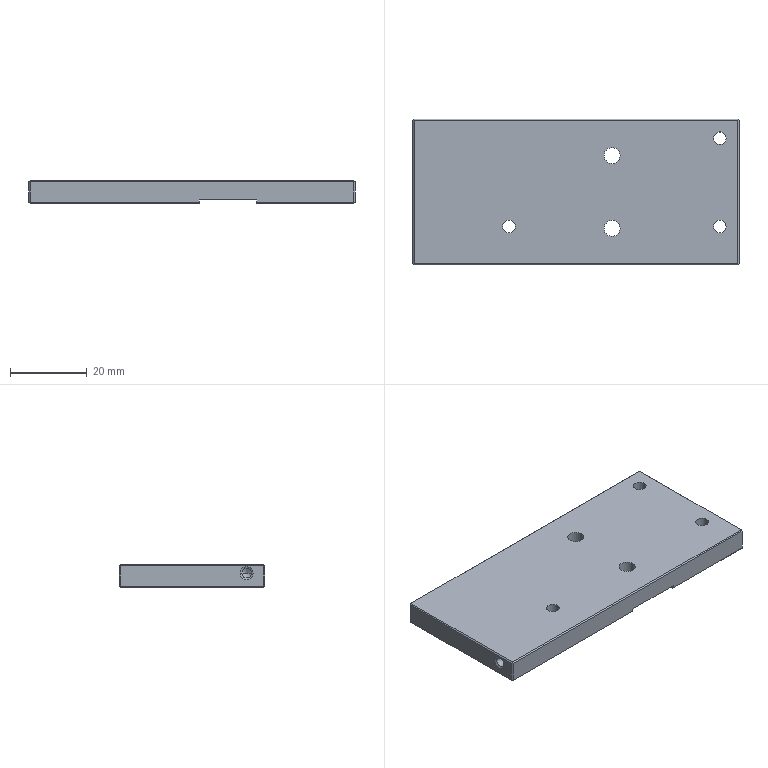Part | NX | 1 solid | 52 faces | box 85 x 38 x 6 mm | volume 18440 mm3 | plane 24 | cone 14 | cylinder 14 | commonest cylinder face diameters 3.3 x6 2.5 x4 4.2 x4
STEP:
#1=CARTESIAN_POINT('',(-230.3,275.,-49.329));
#2=VERTEX_POINT('',#1);
#3=CARTESIAN_POINT('',(-230.3,275.,-54.729));
#4=VERTEX_POINT('',#3);
#5=CARTESIAN_POINT('',(-230.3,275.,-52.029));
#6=DIRECTION('',(0.,0.,-1.));
#7=VECTOR('',#6,1000.);
#8=LINE('',#5,#7);
#9=EDGE_CURVE('',#2,#4,#8,.T.);
#10=ORIENTED_EDGE('',*,*,#9,.T.);
#11=CARTESIAN_POINT('',(-255.6,275.,-54.729));
#12=VERTEX_POINT('',#11);
#13=CARTESIAN_POINT('',(-242.8,275.,-54.729));
#14=DIRECTION('',(-1.,0.,0.));
#15=VECTOR('',#14,1000.);
#16=LINE('',#13,#15);
#17=EDGE_CURVE('',#4,#12,#16,.T.);
#18=ORIENTED_EDGE('',*,*,#17,.T.);
#19=CARTESIAN_POINT('',(-255.6,275.,-54.029));
#20=VERTEX_POINT('',#19);
#21=CARTESIAN_POINT('',(-255.6,275.,-49.029));
#22=DIRECTION('',(0.,0.,-1.));
#23=VECTOR('',#22,1000.);
#24=LINE('',#21,#23);
#25=EDGE_CURVE('',#20,#12,#24,.T.);
#26=ORIENTED_EDGE('',*,*,#25,.F.);
#27=CARTESIAN_POINT('',(-270.6,275.,-54.029));
#28=VERTEX_POINT('',#27);
#29=CARTESIAN_POINT('',(-269.907,275.,-54.029));
#30=DIRECTION('',(1.,0.,0.));
#31=VECTOR('',#30,1000.);
#32=LINE('',#29,#31);
#33=EDGE_CURVE('',#28,#20,#32,.T.);
#34=ORIENTED_EDGE('',*,*,#33,.F.);
#35=CARTESIAN_POINT('',(-270.6,275.,-54.729));
#36=VERTEX_POINT('',#35);
#37=CARTESIAN_POINT('',(-270.6,275.,-49.029));
#38=DIRECTION('',(0.,0.,1.));
#39=VECTOR('',#38,1000.);
#40=LINE('',#37,#39);
#41=EDGE_CURVE('',#36,#28,#40,.T.);
#42=ORIENTED_EDGE('',*,*,#41,.F.);
#43=CARTESIAN_POINT('',(-314.7,275.,-54.729));
#44=VERTEX_POINT('',#43);
#45=CARTESIAN_POINT('',(-292.8,275.,-54.729));
#46=DIRECTION('',(-1.,0.,0.));
#47=VECTOR('',#46,1000.);
#48=LINE('',#45,#47);
#49=EDGE_CURVE('',#36,#44,#48,.T.);
#50=ORIENTED_EDGE('',*,*,#49,.T.);
#51=CARTESIAN_POINT('',(-314.7,275.,-49.329));
#52=VERTEX_POINT('',#51);
#53=CARTESIAN_POINT('',(-314.7,275.,-52.029));
#54=DIRECTION('',(0.,0.,-1.));
#55=VECTOR('',#54,1000.);
#56=LINE('',#53,#55);
#57=EDGE_CURVE('',#52,#44,#56,.T.);
#58=ORIENTED_EDGE('',*,*,#57,.F.);
#59=CARTESIAN_POINT('',(-272.5,275.,-49.329));
#60=DIRECTION('',(-1.,0.,0.));
#61=VECTOR('',#60,1000.);
#62=LINE('',#59,#61);
#63=EDGE_CURVE('',#2,#52,#62,.T.);
#64=ORIENTED_EDGE('',*,*,#63,.F.);
#65=EDGE_LOOP('',(#10,#18,#26,#34,#42,#50,#58,#64));
#66=FACE_BOUND('',#65,.T.);
#67=CARTESIAN_POINT('',(-230.,275.,-49.029));
#68=DIRECTION('',(0.,1.,0.));
#69=DIRECTION('',(0.,0.,-1.));
#70=AXIS2_PLACEMENT_3D('',#67,#68,#69);
#71=PLANE('',#70);
#72=ADVANCED_FACE('',(#66),#71,.T.);
#73=CARTESIAN_POINT('',(-230.,237.3,-49.329));
#74=VERTEX_POINT('',#73);
#75=CARTESIAN_POINT('',(-230.,237.3,-54.729));
#76=VERTEX_POINT('',#75);
#77=CARTESIAN_POINT('',(-230.,237.3,-52.029));
#78=DIRECTION('',(0.,0.,-1.));
#79=VECTOR('',#78,1000.);
#80=LINE('',#77,#79);
#81=EDGE_CURVE('',#74,#76,#80,.T.);
#82=ORIENTED_EDGE('',*,*,#81,.T.);
#83=CARTESIAN_POINT('',(-230.,274.7,-54.729));
#84=VERTEX_POINT('',#83);
#85=CARTESIAN_POINT('',(-230.,256.,-54.729));
#86=DIRECTION('',(0.,1.,0.));
#87=VECTOR('',#86,1000.);
#88=LINE('',#85,#87);
#89=EDGE_CURVE('',#76,#84,#88,.T.);
#90=ORIENTED_EDGE('',*,*,#89,.T.);
#91=CARTESIAN_POINT('',(-230.,274.7,-49.329));
#92=VERTEX_POINT('',#91);
#93=CARTESIAN_POINT('',(-230.,274.7,-52.029));
#94=DIRECTION('',(0.,0.,-1.));
#95=VECTOR('',#94,1000.);
#96=LINE('',#93,#95);
#97=EDGE_CURVE('',#92,#84,#96,.T.);
#98=ORIENTED_EDGE('',*,*,#97,.F.);
#99=CARTESIAN_POINT('',(-230.,256.,-49.329));
#100=DIRECTION('',(0.,1.,0.));
#101=VECTOR('',#100,1000.);
#102=LINE('',#99,#101);
#103=EDGE_CURVE('',#74,#92,#102,.T.);
#104=ORIENTED_EDGE('',*,*,#103,.F.);
#105=EDGE_LOOP('',(#82,#90,#98,#104));
#106=FACE_BOUND('',#105,.T.);
#107=CARTESIAN_POINT('',(-230.,237.,-49.029));
#108=DIRECTION('',(1.,0.,0.));
#109=DIRECTION('',(0.,0.,1.));
#110=AXIS2_PLACEMENT_3D('',#107,#108,#109);
#111=PLANE('',#110);
#112=ADVANCED_FACE('',(#106),#111,.T.);
#113=CARTESIAN_POINT('',(-314.7,237.,-49.329));
#114=VERTEX_POINT('',#113);
#115=CARTESIAN_POINT('',(-314.7,237.,-54.729));
#116=VERTEX_POINT('',#115);
#117=CARTESIAN_POINT('',(-314.7,237.,-52.029));
#118=DIRECTION('',(0.,0.,-1.));
#119=VECTOR('',#118,1000.);
#120=LINE('',#117,#119);
#121=EDGE_CURVE('',#114,#116,#120,.T.);
#122=ORIENTED_EDGE('',*,*,#121,.T.);
#123=CARTESIAN_POINT('',(-270.6,237.,-54.729));
#124=VERTEX_POINT('',#123);
#125=CARTESIAN_POINT('',(-292.8,237.,-54.729));
#126=DIRECTION('',(1.,0.,0.));
#127=VECTOR('',#126,1000.);
#128=LINE('',#125,#127);
#129=EDGE_CURVE('',#116,#124,#128,.T.);
#130=ORIENTED_EDGE('',*,*,#129,.T.);
#131=CARTESIAN_POINT('',(-270.6,237.,-54.029));
#132=VERTEX_POINT('',#131);
#133=CARTESIAN_POINT('',(-270.6,237.,-49.029));
#134=DIRECTION('',(0.,0.,-1.));
#135=VECTOR('',#134,1000.);
#136=LINE('',#133,#135);
#137=EDGE_CURVE('',#132,#124,#136,.T.);
#138=ORIENTED_EDGE('',*,*,#137,.F.);
#139=CARTESIAN_POINT('',(-255.6,237.,-54.029));
#140=VERTEX_POINT('',#139);
#141=CARTESIAN_POINT('',(-269.907,237.,-54.029));
#142=DIRECTION('',(-1.,0.,0.));
#143=VECTOR('',#142,1000.);
#144=LINE('',#141,#143);
#145=EDGE_CURVE('',#140,#132,#144,.T.);
#146=ORIENTED_EDGE('',*,*,#145,.F.);
#147=CARTESIAN_POINT('',(-255.6,237.,-54.729));
#148=VERTEX_POINT('',#147);
#149=CARTESIAN_POINT('',(-255.6,237.,-49.029));
#150=DIRECTION('',(0.,0.,1.));
#151=VECTOR('',#150,1000.);
#152=LINE('',#149,#151);
#153=EDGE_CURVE('',#148,#140,#152,.T.);
#154=ORIENTED_EDGE('',*,*,#153,.F.);
#155=CARTESIAN_POINT('',(-230.3,237.,-54.729));
#156=VERTEX_POINT('',#155);
#157=CARTESIAN_POINT('',(-242.8,237.,-54.729));
#158=DIRECTION('',(1.,0.,0.));
#159=VECTOR('',#158,1000.);
#160=LINE('',#157,#159);
#161=EDGE_CURVE('',#148,#156,#160,.T.);
#162=ORIENTED_EDGE('',*,*,#161,.T.);
#163=CARTESIAN_POINT('',(-230.3,237.,-49.329));
#164=VERTEX_POINT('',#163);
#165=CARTESIAN_POINT('',(-230.3,237.,-52.029));
#166=DIRECTION('',(0.,0.,-1.));
#167=VECTOR('',#166,1000.);
#168=LINE('',#165,#167);
#169=EDGE_CURVE('',#164,#156,#168,.T.);
#170=ORIENTED_EDGE('',*,*,#169,.F.);
#171=CARTESIAN_POINT('',(-272.5,237.,-49.329));
#172=DIRECTION('',(1.,0.,0.));
#173=VECTOR('',#172,1000.);
#174=LINE('',#171,#173);
#175=EDGE_CURVE('',#114,#164,#174,.T.);
#176=ORIENTED_EDGE('',*,*,#175,.F.);
#177=EDGE_LOOP('',(#122,#130,#138,#146,#154,#162,#170,#176));
#178=FACE_BOUND('',#177,.T.);
#179=CARTESIAN_POINT('',(-315.,237.,-49.029));
#180=DIRECTION('',(0.,-1.,0.));
#181=DIRECTION('',(0.,0.,-1.));
#182=AXIS2_PLACEMENT_3D('',#179,#180,#181);
#183=PLANE('',#182);
#184=ADVANCED_FACE('',(#178),#183,.T.);
#185=CARTESIAN_POINT('',(-315.,274.7,-49.329));
#186=VERTEX_POINT('',#185);
#187=CARTESIAN_POINT('',(-315.,237.3,-49.329));
#188=VERTEX_POINT('',#187);
#189=CARTESIAN_POINT('',(-315.,256.,-49.329));
#190=DIRECTION('',(0.,-1.,0.));
#191=VECTOR('',#190,1000.);
#192=LINE('',#189,#191);
#193=EDGE_CURVE('',#186,#188,#192,.T.);
#194=ORIENTED_EDGE('',*,*,#193,.F.);
#195=CARTESIAN_POINT('',(-315.,274.7,-54.729));
#196=VERTEX_POINT('',#195);
#197=CARTESIAN_POINT('',(-315.,274.7,-52.029));
#198=DIRECTION('',(0.,0.,-1.));
#199=VECTOR('',#198,1000.);
#200=LINE('',#197,#199);
#201=EDGE_CURVE('',#186,#196,#200,.T.);
#202=ORIENTED_EDGE('',*,*,#201,.T.);
#203=CARTESIAN_POINT('',(-315.,237.3,-54.729));
#204=VERTEX_POINT('',#203);
#205=CARTESIAN_POINT('',(-315.,256.,-54.729));
#206=DIRECTION('',(0.,-1.,0.));
#207=VECTOR('',#206,1000.);
#208=LINE('',#205,#207);
#209=EDGE_CURVE('',#196,#204,#208,.T.);
#210=ORIENTED_EDGE('',*,*,#209,.T.);
#211=CARTESIAN_POINT('',(-315.,237.3,-52.029));
#212=DIRECTION('',(0.,0.,-1.));
#213=VECTOR('',#212,1000.);
#214=LINE('',#211,#213);
#215=EDGE_CURVE('',#188,#204,#214,.T.);
#216=ORIENTED_EDGE('',*,*,#215,.F.);
#217=EDGE_LOOP('',(#194,#202,#210,#216));
#218=FACE_BOUND('',#217,.T.);
#219=CARTESIAN_POINT('',(-315.,243.45,-51.279));
#220=VERTEX_POINT('',#219);
#221=CARTESIAN_POINT('',(-315.,240.05,-51.279));
#222=VERTEX_POINT('',#221);
#223=CARTESIAN_POINT('',(-315.,241.75,-51.279));
#224=DIRECTION('',(-1.,0.,0.));
#225=DIRECTION('',(0.,-1.,0.));
#226=AXIS2_PLACEMENT_3D('',#223,#224,#225);
#227=CIRCLE('',#226,1.7);
#228=EDGE_CURVE('',#220,#222,#227,.T.);
#229=ORIENTED_EDGE('',*,*,#228,.F.);
#230=CARTESIAN_POINT('',(-315.,241.75,-51.279));
#231=DIRECTION('',(-1.,0.,0.));
#232=DIRECTION('',(0.,-1.,0.));
#233=AXIS2_PLACEMENT_3D('',#230,#231,#232);
#234=CIRCLE('',#233,1.7);
#235=EDGE_CURVE('',#222,#220,#234,.T.);
#236=ORIENTED_EDGE('',*,*,#235,.F.);
#237=EDGE_LOOP('',(#229,#236));
#238=FACE_BOUND('',#237,.T.);
#239=CARTESIAN_POINT('',(-315.,275.,-49.029));
#240=DIRECTION('',(-1.,0.,0.));
#241=DIRECTION('',(0.,0.,1.));
#242=AXIS2_PLACEMENT_3D('',#239,#240,#241);
#243=PLANE('',#242);
#244=ADVANCED_FACE('',(#218,#238),#243,.T.);
#245=ORIENTED_EDGE('',*,*,#25,.T.);
#246=CARTESIAN_POINT('',(-255.6,274.7,-55.029));
#247=VERTEX_POINT('',#246);
#248=CARTESIAN_POINT('',(-255.6,266.432,-63.297));
#249=DIRECTION('',(0.,0.7071,0.7071));
#250=VECTOR('',#249,1000.);
#251=LINE('',#248,#250);
#252=EDGE_CURVE('',#247,#12,#251,.T.);
#253=ORIENTED_EDGE('',*,*,#252,.F.);
#254=CARTESIAN_POINT('',(-255.6,237.3,-55.029));
#255=VERTEX_POINT('',#254);
#256=CARTESIAN_POINT('',(-255.6,266.432,-55.029));
#257=DIRECTION('',(0.,-1.,0.));
#258=VECTOR('',#257,1000.);
#259=LINE('',#256,#258);
#260=EDGE_CURVE('',#247,#255,#259,.T.);
#261=ORIENTED_EDGE('',*,*,#260,.T.);
#262=CARTESIAN_POINT('',(-255.6,266.432,-84.161));
#263=DIRECTION('',(0.,0.7071,-0.7071));
#264=VECTOR('',#263,1000.);
#265=LINE('',#262,#264);
#266=EDGE_CURVE('',#148,#255,#265,.T.);
#267=ORIENTED_EDGE('',*,*,#266,.F.);
#268=ORIENTED_EDGE('',*,*,#153,.T.);
#269=CARTESIAN_POINT('',(-255.6,233.2,-54.029));
#270=DIRECTION('',(0.,1.,0.));
#271=VECTOR('',#270,1000.);
#272=LINE('',#269,#271);
#273=EDGE_CURVE('',#140,#20,#272,.T.);
#274=ORIENTED_EDGE('',*,*,#273,.T.);
#275=EDGE_LOOP('',(#245,#253,#261,#267,#268,#274));
#276=FACE_BOUND('',#275,.T.);
#277=CARTESIAN_POINT('',(-255.6,233.2,-89.));
#278=DIRECTION('',(1.,0.,0.));
#279=DIRECTION('',(0.,1.,0.));
#280=AXIS2_PLACEMENT_3D('',#277,#278,#279);
#281=PLANE('',#280);
#282=ADVANCED_FACE('',(#276),#281,.F.);
#283=CARTESIAN_POINT('',(-314.74,243.,-51.279));
#284=VERTEX_POINT('',#283);
#285=CARTESIAN_POINT('',(-314.74,240.5,-51.279));
#286=VERTEX_POINT('',#285);
#287=CARTESIAN_POINT('',(-314.74,241.75,-51.279));
#288=DIRECTION('',(-1.,0.,0.));
#289=DIRECTION('',(0.,-1.,0.));
#290=AXIS2_PLACEMENT_3D('',#287,#288,#289);
#291=CIRCLE('',#290,1.25);
#292=EDGE_CURVE('',#284,#286,#291,.T.);
#293=ORIENTED_EDGE('',*,*,#292,.F.);
#294=CARTESIAN_POINT('',(-314.74,243.,-51.279));
#295=DIRECTION('',(-0.5,0.866,0.));
#296=VECTOR('',#295,1000.);
#297=LINE('',#294,#296);
#298=EDGE_CURVE('',#220,#284,#297,.F.);
#299=ORIENTED_EDGE('',*,*,#298,.F.);
#300=ORIENTED_EDGE('',*,*,#228,.T.);
#301=CARTESIAN_POINT('',(-314.74,240.5,-51.279));
#302=DIRECTION('',(-0.5,-0.866,0.));
#303=VECTOR('',#302,1000.);
#304=LINE('',#301,#303);
#305=EDGE_CURVE('',#222,#286,#304,.F.);
#306=ORIENTED_EDGE('',*,*,#305,.T.);
#307=EDGE_LOOP('',(#293,#299,#300,#306));
#308=FACE_BOUND('',#307,.T.);
#309=CARTESIAN_POINT('',(-314.74,241.75,-51.279));
#310=DIRECTION('',(-1.,0.,0.));
#311=DIRECTION('',(0.,-1.,0.));
#312=AXIS2_PLACEMENT_3D('',#309,#310,#311);
#313=CONICAL_SURFACE('',#312,1.25,1.047);
#314=ADVANCED_FACE('',(#308),#313,.F.);
#315=CARTESIAN_POINT('',(-306.,243.,-51.279));
#316=VERTEX_POINT('',#315);
#317=CARTESIAN_POINT('',(-306.,240.5,-51.279));
#318=VERTEX_POINT('',#317);
#319=CARTESIAN_POINT('',(-306.,241.75,-51.279));
#320=DIRECTION('',(-1.,0.,0.));
#321=DIRECTION('',(0.,-1.,0.));
#322=AXIS2_PLACEMENT_3D('',#319,#320,#321);
#323=CIRCLE('',#322,1.25);
#324=EDGE_CURVE('',#316,#318,#323,.T.);
#325=ORIENTED_EDGE('',*,*,#324,.T.);
#326=CARTESIAN_POINT('',(-305.249,241.75,-51.279));
#327=VERTEX_POINT('',#326);
#328=CARTESIAN_POINT('',(-306.,240.5,-51.279));
#329=DIRECTION('',(-0.515,-0.8572,0.));
#330=VECTOR('',#329,1000.);
#331=LINE('',#328,#330);
#332=EDGE_CURVE('',#327,#318,#331,.T.);
#333=ORIENTED_EDGE('',*,*,#332,.F.);
#334=CARTESIAN_POINT('',(-306.,243.,-51.279));
#335=DIRECTION('',(-0.515,0.8572,0.));
#336=VECTOR('',#335,1000.);
#337=LINE('',#334,#336);
#338=EDGE_CURVE('',#327,#316,#337,.T.);
#339=ORIENTED_EDGE('',*,*,#338,.T.);
#340=EDGE_LOOP('',(#325,#333,#339));
#341=FACE_BOUND('',#340,.T.);
#342=CARTESIAN_POINT('',(-306.,241.75,-51.279));
#343=DIRECTION('',(-1.,0.,0.));
#344=DIRECTION('',(0.,-1.,0.));
#345=AXIS2_PLACEMENT_3D('',#342,#343,#344);
#346=CONICAL_SURFACE('',#345,1.25,1.03);
#347=ADVANCED_FACE('',(#341),#346,.F.);
#348=CARTESIAN_POINT('',(-309.,243.,-51.279));
#349=VERTEX_POINT('',#348);
#350=CARTESIAN_POINT('',(-309.,240.5,-51.279));
#351=VERTEX_POINT('',#350);
#352=CARTESIAN_POINT('',(-309.,241.75,-51.279));
#353=DIRECTION('',(-1.,0.,0.));
#354=DIRECTION('',(0.,-1.,0.));
#355=AXIS2_PLACEMENT_3D('',#352,#353,#354);
#356=CIRCLE('',#355,1.25);
#357=EDGE_CURVE('',#349,#351,#356,.T.);
#358=ORIENTED_EDGE('',*,*,#357,.T.);
#359=CARTESIAN_POINT('',(-315.,240.5,-51.279));
#360=DIRECTION('',(-1.,0.,0.));
#361=VECTOR('',#360,1000.);
#362=LINE('',#359,#361);
#363=EDGE_CURVE('',#351,#318,#362,.F.);
#364=ORIENTED_EDGE('',*,*,#363,.T.);
#365=ORIENTED_EDGE('',*,*,#324,.F.);
#366=CARTESIAN_POINT('',(-315.,243.,-51.279));
#367=DIRECTION('',(-1.,0.,0.));
#368=VECTOR('',#367,1000.);
#369=LINE('',#366,#368);
#370=EDGE_CURVE('',#349,#316,#369,.F.);
#371=ORIENTED_EDGE('',*,*,#370,.F.);
#372=EDGE_LOOP('',(#358,#364,#365,#371));
#373=FACE_BOUND('',#372,.T.);
#374=CARTESIAN_POINT('',(-315.,241.75,-51.279));
#375=DIRECTION('',(-1.,0.,0.));
#376=DIRECTION('',(0.,-1.,0.));
#377=AXIS2_PLACEMENT_3D('',#374,#375,#376);
#378=CYLINDRICAL_SURFACE('',#377,1.25);
#379=ADVANCED_FACE('',(#373),#378,.F.);
#380=ORIENTED_EDGE('',*,*,#292,.T.);
#381=CARTESIAN_POINT('',(-315.,240.5,-51.279));
#382=DIRECTION('',(-1.,0.,0.));
#383=VECTOR('',#382,1000.);
#384=LINE('',#381,#383);
#385=EDGE_CURVE('',#286,#351,#384,.F.);
#386=ORIENTED_EDGE('',*,*,#385,.T.);
#387=ORIENTED_EDGE('',*,*,#357,.F.);
#388=CARTESIAN_POINT('',(-315.,243.,-51.279));
#389=DIRECTION('',(-1.,0.,0.));
#390=VECTOR('',#389,1000.);
#391=LINE('',#388,#390);
#392=EDGE_CURVE('',#284,#349,#391,.F.);
#393=ORIENTED_EDGE('',*,*,#392,.F.);
#394=EDGE_LOOP('',(#380,#386,#387,#393));
#395=FACE_BOUND('',#394,.T.);
#396=CARTESIAN_POINT('',(-315.,241.75,-51.279));
#397=DIRECTION('',(-1.,0.,0.));
#398=DIRECTION('',(0.,-1.,0.));
#399=AXIS2_PLACEMENT_3D('',#396,#397,#398);
#400=CYLINDRICAL_SURFACE('',#399,1.25);
#401=ADVANCED_FACE('',(#395),#400,.F.);
#402=ORIENTED_EDGE('',*,*,#57,.T.);
#403=CARTESIAN_POINT('',(-314.85,274.85,-54.879));
#404=VERTEX_POINT('',#403);
#405=CARTESIAN_POINT('',(-323.268,266.432,-63.297));
#406=DIRECTION('',(-0.5774,-0.5774,-0.5774));
#407=VECTOR('',#406,1000.);
#408=LINE('',#405,#407);
#409=EDGE_CURVE('',#44,#404,#408,.T.);
#410=ORIENTED_EDGE('',*,*,#409,.T.);
#411=CARTESIAN_POINT('',(-323.268,266.432,-46.461));
#412=DIRECTION('',(-0.5774,-0.5774,0.5774));
#413=VECTOR('',#412,1000.);
#414=LINE('',#411,#413);
#415=EDGE_CURVE('',#404,#196,#414,.T.);
#416=ORIENTED_EDGE('',*,*,#415,.T.);
#417=ORIENTED_EDGE('',*,*,#201,.F.);
#418=CARTESIAN_POINT('',(-314.85,274.85,-49.179));
#419=VERTEX_POINT('',#418);
#420=CARTESIAN_POINT('',(-323.268,266.432,-57.597));
#421=DIRECTION('',(-0.5774,-0.5774,-0.5774));
#422=VECTOR('',#421,1000.);
#423=LINE('',#420,#422);
#424=EDGE_CURVE('',#419,#186,#423,.T.);
#425=ORIENTED_EDGE('',*,*,#424,.F.);
#426=CARTESIAN_POINT('',(-323.268,266.432,-40.761));
#427=DIRECTION('',(-0.5774,-0.5774,0.5774));
#428=VECTOR('',#427,1000.);
#429=LINE('',#426,#428);
#430=EDGE_CURVE('',#52,#419,#429,.T.);
#431=ORIENTED_EDGE('',*,*,#430,.F.);
#432=EDGE_LOOP('',(#402,#410,#416,#417,#425,#431));
#433=FACE_BOUND('',#432,.T.);
#434=CARTESIAN_POINT('',(-314.85,274.85,-52.029));
#435=DIRECTION('',(0.7071,-0.7071,0.));
#436=DIRECTION('',(0.,0.,-1.));
#437=AXIS2_PLACEMENT_3D('',#434,#435,#436);
#438=PLANE('',#437);
#439=ADVANCED_FACE('',(#433),#438,.F.);
#440=ORIENTED_EDGE('',*,*,#121,.F.);
#441=CARTESIAN_POINT('',(-314.85,237.15,-49.179));
#442=VERTEX_POINT('',#441);
#443=CARTESIAN_POINT('',(-344.132,266.432,-19.897));
#444=DIRECTION('',(-0.5774,0.5774,0.5774));
#445=VECTOR('',#444,1000.);
#446=LINE('',#443,#445);
#447=EDGE_CURVE('',#114,#442,#446,.T.);
#448=ORIENTED_EDGE('',*,*,#447,.T.);
#449=CARTESIAN_POINT('',(-314.7,237.,-49.029));
#450=DIRECTION('',(0.5774,-0.5774,0.5774));
#451=VECTOR('',#450,1000.);
#452=LINE('',#449,#451);
#453=EDGE_CURVE('',#188,#442,#452,.T.);
#454=ORIENTED_EDGE('',*,*,#453,.F.);
#455=ORIENTED_EDGE('',*,*,#215,.T.);
#456=CARTESIAN_POINT('',(-314.85,237.15,-54.879));
#457=VERTEX_POINT('',#456);
#458=CARTESIAN_POINT('',(-320.7,243.,-49.029));
#459=DIRECTION('',(0.5774,-0.5774,-0.5774));
#460=VECTOR('',#459,1000.);
#461=LINE('',#458,#460);
#462=EDGE_CURVE('',#204,#457,#461,.T.);
#463=ORIENTED_EDGE('',*,*,#462,.T.);
#464=CARTESIAN_POINT('',(-344.132,266.432,-84.161));
#465=DIRECTION('',(0.5774,-0.5774,0.5774));
#466=VECTOR('',#465,1000.);
#467=LINE('',#464,#466);
#468=EDGE_CURVE('',#457,#116,#467,.T.);
#469=ORIENTED_EDGE('',*,*,#468,.T.);
#470=EDGE_LOOP('',(#440,#448,#454,#455,#463,#469));
#471=FACE_BOUND('',#470,.T.);
#472=CARTESIAN_POINT('',(-314.85,237.15,-52.029));
#473=DIRECTION('',(-0.7071,-0.7071,0.));
#474=DIRECTION('',(-0.7071,0.7071,0.));
#475=AXIS2_PLACEMENT_3D('',#472,#473,#474);
#476=PLANE('',#475);
#477=ADVANCED_FACE('',(#471),#476,.T.);
#478=ORIENTED_EDGE('',*,*,#81,.F.);
#479=CARTESIAN_POINT('',(-230.15,237.15,-49.179));
#480=VERTEX_POINT('',#479);
#481=CARTESIAN_POINT('',(-200.868,266.432,-78.461));
#482=DIRECTION('',(-0.5774,-0.5774,0.5774));
#483=VECTOR('',#482,1000.);
#484=LINE('',#481,#483);
#485=EDGE_CURVE('',#74,#480,#484,.T.);
#486=ORIENTED_EDGE('',*,*,#485,.T.);
#487=CARTESIAN_POINT('',(-200.868,266.432,-19.897));
#488=DIRECTION('',(0.5774,0.5774,0.5774));
#489=VECTOR('',#488,1000.);
#490=LINE('',#487,#489);
#491=EDGE_CURVE('',#164,#480,#490,.T.);
#492=ORIENTED_EDGE('',*,*,#491,.F.);
#493=ORIENTED_EDGE('',*,*,#169,.T.);
#494=CARTESIAN_POINT('',(-230.15,237.15,-54.879));
#495=VERTEX_POINT('',#494);
#496=CARTESIAN_POINT('',(-200.868,266.432,-84.161));
#497=DIRECTION('',(0.5774,0.5774,-0.5774));
#498=VECTOR('',#497,1000.);
#499=LINE('',#496,#498);
#500=EDGE_CURVE('',#156,#495,#499,.T.);
#501=ORIENTED_EDGE('',*,*,#500,.T.);
#502=CARTESIAN_POINT('',(-200.868,266.432,-25.597));
#503=DIRECTION('',(-0.5774,-0.5774,-0.5774));
#504=VECTOR('',#503,1000.);
#505=LINE('',#502,#504);
#506=EDGE_CURVE('',#76,#495,#505,.T.);
#507=ORIENTED_EDGE('',*,*,#506,.F.);
#508=EDGE_LOOP('',(#478,#486,#492,#493,#501,#507));
#509=FACE_BOUND('',#508,.T.);
#510=CARTESIAN_POINT('',(-230.15,237.15,-52.029));
#511=DIRECTION('',(0.7071,-0.7071,0.));
#512=DIRECTION('',(0.,0.,-1.));
#513=AXIS2_PLACEMENT_3D('',#510,#511,#512);
#514=PLANE('',#513);
#515=ADVANCED_FACE('',(#509),#514,.T.);
#516=ORIENTED_EDGE('',*,*,#9,.F.);
#517=CARTESIAN_POINT('',(-230.15,274.85,-49.179));
#518=VERTEX_POINT('',#517);
#519=CARTESIAN_POINT('',(-221.732,266.432,-40.761));
#520=DIRECTION('',(-0.5774,0.5774,-0.5774));
#521=VECTOR('',#520,1000.);
#522=LINE('',#519,#521);
#523=EDGE_CURVE('',#518,#2,#522,.T.);
#524=ORIENTED_EDGE('',*,*,#523,.F.);
#525=CARTESIAN_POINT('',(-230.3,275.,-49.029));
#526=DIRECTION('',(-0.5774,0.5774,0.5774));
#527=VECTOR('',#526,1000.);
#528=LINE('',#525,#527);
#529=EDGE_CURVE('',#92,#518,#528,.T.);
#530=ORIENTED_EDGE('',*,*,#529,.F.);
#531=ORIENTED_EDGE('',*,*,#97,.T.);
#532=CARTESIAN_POINT('',(-230.15,274.85,-54.879));
#533=VERTEX_POINT('',#532);
#534=CARTESIAN_POINT('',(-224.3,269.,-49.029));
#535=DIRECTION('',(-0.5774,0.5774,-0.5774));
#536=VECTOR('',#535,1000.);
#537=LINE('',#534,#536);
#538=EDGE_CURVE('',#84,#533,#537,.T.);
#539=ORIENTED_EDGE('',*,*,#538,.T.);
#540=CARTESIAN_POINT('',(-221.732,266.432,-63.297));
#541=DIRECTION('',(0.5774,-0.5774,-0.5774));
#542=VECTOR('',#541,1000.);
#543=LINE('',#540,#542);
#544=EDGE_CURVE('',#4,#533,#543,.T.);
#545=ORIENTED_EDGE('',*,*,#544,.F.);
#546=EDGE_LOOP('',(#516,#524,#530,#531,#539,#545));
#547=FACE_BOUND('',#546,.T.);
#548=CARTESIAN_POINT('',(-230.15,274.85,-52.029));
#549=DIRECTION('',(0.7071,0.7071,0.));
#550=DIRECTION('',(0.,0.,-1.));
#551=AXIS2_PLACEMENT_3D('',#548,#549,#550);
#552=PLANE('',#551);
#553=ADVANCED_FACE('',(#547),#552,.T.);
#554=ORIENTED_EDGE('',*,*,#363,.F.);
#555=CARTESIAN_POINT('',(-309.,241.75,-51.279));
#556=DIRECTION('',(-1.,0.,0.));
#557=DIRECTION('',(0.,-1.,0.));
#558=AXIS2_PLACEMENT_3D('',#555,#556,#557);
#559=CIRCLE('',#558,1.25);
#560=EDGE_CURVE('',#351,#349,#559,.T.);
#561=ORIENTED_EDGE('',*,*,#560,.T.);
#562=ORIENTED_EDGE('',*,*,#370,.T.);
#563=CARTESIAN_POINT('',(-306.,241.75,-51.279));
#564=DIRECTION('',(-1.,0.,0.));
#565=DIRECTION('',(0.,-1.,0.));
#566=AXIS2_PLACEMENT_3D('',#563,#564,#565);
#567=CIRCLE('',#566,1.25);
#568=EDGE_CURVE('',#318,#316,#567,.T.);
#569=ORIENTED_EDGE('',*,*,#568,.F.);
#570=EDGE_LOOP('',(#554,#561,#562,#569));
#571=FACE_BOUND('',#570,.T.);
#572=CARTESIAN_POINT('',(-315.,241.75,-51.279));
#573=DIRECTION('',(-1.,0.,0.));
#574=DIRECTION('',(0.,-1.,0.));
#575=AXIS2_PLACEMENT_3D('',#572,#573,#574);
#576=CYLINDRICAL_SURFACE('',#575,1.25);
#577=ADVANCED_FACE('',(#571),#576,.F.);
#578=ORIENTED_EDGE('',*,*,#338,.F.);
#579=ORIENTED_EDGE('',*,*,#332,.T.);
#580=ORIENTED_EDGE('',*,*,#568,.T.);
#581=EDGE_LOOP('',(#578,#579,#580));
#582=FACE_BOUND('',#581,.T.);
#583=CARTESIAN_POINT('',(-306.,241.75,-51.279));
#584=DIRECTION('',(-1.,0.,0.));
#585=DIRECTION('',(0.,-1.,0.));
#586=AXIS2_PLACEMENT_3D('',#583,#584,#585);
#587=CONICAL_SURFACE('',#586,1.25,1.03);
#588=ADVANCED_FACE('',(#582),#587,.F.);
#589=ORIENTED_EDGE('',*,*,#305,.F.);
#590=ORIENTED_EDGE('',*,*,#235,.T.);
#591=ORIENTED_EDGE('',*,*,#298,.T.);
#592=CARTESIAN_POINT('',(-314.74,241.75,-51.279));
#593=DIRECTION('',(-1.,0.,0.));
#594=DIRECTION('',(0.,-1.,0.));
#595=AXIS2_PLACEMENT_3D('',#592,#593,#594);
#596=CIRCLE('',#595,1.25);
#597=EDGE_CURVE('',#286,#284,#596,.T.);
#598=ORIENTED_EDGE('',*,*,#597,.F.);
#599=EDGE_LOOP('',(#589,#590,#591,#598));
#600=FACE_BOUND('',#599,.T.);
#601=CARTESIAN_POINT('',(-314.74,241.75,-51.279));
#602=DIRECTION('',(-1.,0.,0.));
#603=DIRECTION('',(0.,-1.,0.));
#604=AXIS2_PLACEMENT_3D('',#601,#602,#603);
#605=CONICAL_SURFACE('',#604,1.25,1.047);
#606=ADVANCED_FACE('',(#600),#605,.F.);
#607=ORIENTED_EDGE('',*,*,#385,.F.);
#608=ORIENTED_EDGE('',*,*,#597,.T.);
#609=ORIENTED_EDGE('',*,*,#392,.T.);
#610=ORIENTED_EDGE('',*,*,#560,.F.);
#611=EDGE_LOOP('',(#607,#608,#609,#610));
#612=FACE_BOUND('',#611,.T.);
#613=CARTESIAN_POINT('',(-315.,241.75,-51.279));
#614=DIRECTION('',(-1.,0.,0.));
#615=DIRECTION('',(0.,-1.,0.));
#616=AXIS2_PLACEMENT_3D('',#613,#614,#615);
#617=CYLINDRICAL_SURFACE('',#616,1.25);
#618=ADVANCED_FACE('',(#612),#617,.F.);
#619=CARTESIAN_POINT('',(-314.7,237.3,-55.029));
#620=VERTEX_POINT('',#619);
#621=CARTESIAN_POINT('',(-270.6,237.3,-55.029));
#622=VERTEX_POINT('',#621);
#623=CARTESIAN_POINT('',(-292.8,237.3,-55.029));
#624=DIRECTION('',(1.,0.,0.));
#625=VECTOR('',#624,1000.);
#626=LINE('',#623,#625);
#627=EDGE_CURVE('',#620,#622,#626,.T.);
#628=ORIENTED_EDGE('',*,*,#627,.F.);
#629=CARTESIAN_POINT('',(-314.7,274.7,-55.029));
#630=VERTEX_POINT('',#629);
#631=CARTESIAN_POINT('',(-314.7,256.,-55.029));
#632=DIRECTION('',(0.,-1.,0.));
#633=VECTOR('',#632,1000.);
#634=LINE('',#631,#633);
#635=EDGE_CURVE('',#630,#620,#634,.T.);
#636=ORIENTED_EDGE('',*,*,#635,.F.);
#637=CARTESIAN_POINT('',(-270.6,274.7,-55.029));
#638=VERTEX_POINT('',#637);
#639=CARTESIAN_POINT('',(-292.8,274.7,-55.029));
#640=DIRECTION('',(-1.,0.,0.));
#641=VECTOR('',#640,1000.);
#642=LINE('',#639,#641);
#643=EDGE_CURVE('',#638,#630,#642,.T.);
#644=ORIENTED_EDGE('',*,*,#643,.F.);
#645=CARTESIAN_POINT('',(-270.6,266.432,-55.029));
#646=DIRECTION('',(0.,1.,0.));
#647=VECTOR('',#646,1000.);
#648=LINE('',#645,#647);
#649=EDGE_CURVE('',#622,#638,#648,.T.);
#650=ORIENTED_EDGE('',*,*,#649,.F.);
#651=EDGE_LOOP('',(#628,#636,#644,#650));
#652=FACE_BOUND('',#651,.T.);
#653=CARTESIAN_POINT('',(-287.685,247.,-55.029));
#654=VERTEX_POINT('',#653);
#655=CARTESIAN_POINT('',(-292.315,247.,-55.029));
#656=VERTEX_POINT('',#655);
#657=CARTESIAN_POINT('',(-290.,247.,-55.029));
#658=DIRECTION('',(0.,0.,-1.));
#659=DIRECTION('',(-1.,0.,0.));
#660=AXIS2_PLACEMENT_3D('',#657,#658,#659);
#661=CIRCLE('',#660,2.315);
#662=EDGE_CURVE('',#654,#656,#661,.T.);
#663=ORIENTED_EDGE('',*,*,#662,.F.);
#664=CARTESIAN_POINT('',(-290.,247.,-55.029));
#665=DIRECTION('',(0.,0.,-1.));
#666=DIRECTION('',(-1.,0.,0.));
#667=AXIS2_PLACEMENT_3D('',#664,#665,#666);
#668=CIRCLE('',#667,2.315);
#669=EDGE_CURVE('',#656,#654,#668,.T.);
#670=ORIENTED_EDGE('',*,*,#669,.F.);
#671=EDGE_LOOP('',(#663,#670));
#672=FACE_BOUND('',#671,.T.);
#673=CARTESIAN_POINT('',(-269.907,266.432,-55.029));
#674=DIRECTION('',(0.,0.,-1.));
#675=DIRECTION('',(0.,-1.,0.));
#676=AXIS2_PLACEMENT_3D('',#673,#674,#675);
#677=PLANE('',#676);
#678=ADVANCED_FACE('',(#652,#672),#677,.T.);
#679=CARTESIAN_POINT('',(-233.35,270.,-54.645));
#680=VERTEX_POINT('',#679);
#681=CARTESIAN_POINT('',(-236.65,270.,-54.645));
#682=VERTEX_POINT('',#681);
#683=CARTESIAN_POINT('',(-235.,270.,-54.645));
#684=DIRECTION('',(0.,0.,-1.));
#685=DIRECTION('',(-1.,0.,0.));
#686=AXIS2_PLACEMENT_3D('',#683,#684,#685);
#687=CIRCLE('',#686,1.65);
#688=EDGE_CURVE('',#680,#682,#687,.T.);
#689=ORIENTED_EDGE('',*,*,#688,.T.);
#690=CARTESIAN_POINT('',(-236.65,270.,-49.029));
#691=VERTEX_POINT('',#690);
#692=CARTESIAN_POINT('',(-236.65,270.,-55.029));
#693=DIRECTION('',(0.,0.,-1.));
#694=VECTOR('',#693,1000.);
#695=LINE('',#692,#694);
#696=EDGE_CURVE('',#682,#691,#695,.F.);
#697=ORIENTED_EDGE('',*,*,#696,.T.);
#698=CARTESIAN_POINT('',(-233.35,270.,-49.029));
#699=VERTEX_POINT('',#698);
#700=CARTESIAN_POINT('',(-235.,270.,-49.029));
#701=DIRECTION('',(0.,0.,-1.));
#702=DIRECTION('',(-1.,0.,0.));
#703=AXIS2_PLACEMENT_3D('',#700,#701,#702);
#704=CIRCLE('',#703,1.65);
#705=EDGE_CURVE('',#699,#691,#704,.T.);
#706=ORIENTED_EDGE('',*,*,#705,.F.);
#707=CARTESIAN_POINT('',(-233.35,270.,-55.029));
#708=DIRECTION('',(0.,0.,-1.));
#709=VECTOR('',#708,1000.);
#710=LINE('',#707,#709);
#711=EDGE_CURVE('',#680,#699,#710,.F.);
#712=ORIENTED_EDGE('',*,*,#711,.F.);
#713=EDGE_LOOP('',(#689,#697,#706,#712));
#714=FACE_BOUND('',#713,.T.);
#715=CARTESIAN_POINT('',(-235.,270.,-55.029));
#716=DIRECTION('',(0.,0.,-1.));
#717=DIRECTION('',(-1.,0.,0.));
#718=AXIS2_PLACEMENT_3D('',#715,#716,#717);
#719=CYLINDRICAL_SURFACE('',#718,1.65);
#720=ADVANCED_FACE('',(#714),#719,.F.);
#721=ORIENTED_EDGE('',*,*,#688,.F.);
#722=CARTESIAN_POINT('',(-232.685,270.,-55.029));
#723=VERTEX_POINT('',#722);
#724=CARTESIAN_POINT('',(-233.35,270.,-54.645));
#725=DIRECTION('',(0.866,0.,-0.5));
#726=VECTOR('',#725,1000.);
#727=LINE('',#724,#726);
#728=EDGE_CURVE('',#723,#680,#727,.F.);
#729=ORIENTED_EDGE('',*,*,#728,.F.);
#730=CARTESIAN_POINT('',(-237.315,270.,-55.029));
#731=VERTEX_POINT('',#730);
#732=CARTESIAN_POINT('',(-235.,270.,-55.029));
#733=DIRECTION('',(0.,0.,-1.));
#734=DIRECTION('',(-1.,0.,0.));
#735=AXIS2_PLACEMENT_3D('',#732,#733,#734);
#736=CIRCLE('',#735,2.315);
#737=EDGE_CURVE('',#723,#731,#736,.T.);
#738=ORIENTED_EDGE('',*,*,#737,.T.);
#739=CARTESIAN_POINT('',(-236.65,270.,-54.645));
#740=DIRECTION('',(-0.866,0.,-0.5));
#741=VECTOR('',#740,1000.);
#742=LINE('',#739,#741);
#743=EDGE_CURVE('',#731,#682,#742,.F.);
#744=ORIENTED_EDGE('',*,*,#743,.T.);
#745=EDGE_LOOP('',(#721,#729,#738,#744));
#746=FACE_BOUND('',#745,.T.);
#747=CARTESIAN_POINT('',(-235.,270.,-54.645));
#748=DIRECTION('',(0.,0.,-1.));
#749=DIRECTION('',(-1.,0.,0.));
#750=AXIS2_PLACEMENT_3D('',#747,#748,#749);
#751=CONICAL_SURFACE('',#750,1.65,1.047);
#752=ADVANCED_FACE('',(#746),#751,.F.);
#753=CARTESIAN_POINT('',(-233.35,247.,-54.645));
#754=VERTEX_POINT('',#753);
#755=CARTESIAN_POINT('',(-236.65,247.,-54.645));
#756=VERTEX_POINT('',#755);
#757=CARTESIAN_POINT('',(-235.,247.,-54.645));
#758=DIRECTION('',(0.,0.,-1.));
#759=DIRECTION('',(-1.,0.,0.));
#760=AXIS2_PLACEMENT_3D('',#757,#758,#759);
#761=CIRCLE('',#760,1.65);
#762=EDGE_CURVE('',#754,#756,#761,.T.);
#763=ORIENTED_EDGE('',*,*,#762,.T.);
#764=CARTESIAN_POINT('',(-236.65,247.,-49.029));
#765=VERTEX_POINT('',#764);
#766=CARTESIAN_POINT('',(-236.65,247.,-55.029));
#767=DIRECTION('',(0.,0.,-1.));
#768=VECTOR('',#767,1000.);
#769=LINE('',#766,#768);
#770=EDGE_CURVE('',#756,#765,#769,.F.);
#771=ORIENTED_EDGE('',*,*,#770,.T.);
#772=CARTESIAN_POINT('',(-233.35,247.,-49.029));
#773=VERTEX_POINT('',#772);
#774=CARTESIAN_POINT('',(-235.,247.,-49.029));
#775=DIRECTION('',(0.,0.,-1.));
#776=DIRECTION('',(-1.,0.,0.));
#777=AXIS2_PLACEMENT_3D('',#774,#775,#776);
#778=CIRCLE('',#777,1.65);
#779=EDGE_CURVE('',#773,#765,#778,.T.);
#780=ORIENTED_EDGE('',*,*,#779,.F.);
#781=CARTESIAN_POINT('',(-233.35,247.,-55.029));
#782=DIRECTION('',(0.,0.,-1.));
#783=VECTOR('',#782,1000.);
#784=LINE('',#781,#783);
#785=EDGE_CURVE('',#754,#773,#784,.F.);
#786=ORIENTED_EDGE('',*,*,#785,.F.);
#787=EDGE_LOOP('',(#763,#771,#780,#786));
#788=FACE_BOUND('',#787,.T.);
#789=CARTESIAN_POINT('',(-235.,247.,-55.029));
#790=DIRECTION('',(0.,0.,-1.));
#791=DIRECTION('',(-1.,0.,0.));
#792=AXIS2_PLACEMENT_3D('',#789,#790,#791);
#793=CYLINDRICAL_SURFACE('',#792,1.65);
#794=ADVANCED_FACE('',(#788),#793,.F.);
#795=ORIENTED_EDGE('',*,*,#762,.F.);
#796=CARTESIAN_POINT('',(-232.685,247.,-55.029));
#797=VERTEX_POINT('',#796);
#798=CARTESIAN_POINT('',(-233.35,247.,-54.645));
#799=DIRECTION('',(0.866,0.,-0.5));
#800=VECTOR('',#799,1000.);
#801=LINE('',#798,#800);
#802=EDGE_CURVE('',#797,#754,#801,.F.);
#803=ORIENTED_EDGE('',*,*,#802,.F.);
#804=CARTESIAN_POINT('',(-237.315,247.,-55.029));
#805=VERTEX_POINT('',#804);
#806=CARTESIAN_POINT('',(-235.,247.,-55.029));
#807=DIRECTION('',(0.,0.,-1.));
#808=DIRECTION('',(-1.,0.,0.));
#809=AXIS2_PLACEMENT_3D('',#806,#807,#808);
#810=CIRCLE('',#809,2.315);
#811=EDGE_CURVE('',#797,#805,#810,.T.);
#812=ORIENTED_EDGE('',*,*,#811,.T.);
#813=CARTESIAN_POINT('',(-236.65,247.,-54.645));
#814=DIRECTION('',(-0.866,0.,-0.5));
#815=VECTOR('',#814,1000.);
#816=LINE('',#813,#815);
#817=EDGE_CURVE('',#805,#756,#816,.F.);
#818=ORIENTED_EDGE('',*,*,#817,.T.);
#819=EDGE_LOOP('',(#795,#803,#812,#818));
#820=FACE_BOUND('',#819,.T.);
#821=CARTESIAN_POINT('',(-235.,247.,-54.645));
#822=DIRECTION('',(0.,0.,-1.));
#823=DIRECTION('',(-1.,0.,0.));
#824=AXIS2_PLACEMENT_3D('',#821,#822,#823);
#825=CONICAL_SURFACE('',#824,1.65,1.047);
#826=ADVANCED_FACE('',(#820),#825,.F.);
#827=CARTESIAN_POINT('',(-288.35,247.,-54.645));
#828=VERTEX_POINT('',#827);
#829=CARTESIAN_POINT('',(-291.65,247.,-54.645));
#830=VERTEX_POINT('',#829);
#831=CARTESIAN_POINT('',(-290.,247.,-54.645));
#832=DIRECTION('',(0.,0.,-1.));
#833=DIRECTION('',(-1.,0.,0.));
#834=AXIS2_PLACEMENT_3D('',#831,#832,#833);
#835=CIRCLE('',#834,1.65);
#836=EDGE_CURVE('',#828,#830,#835,.T.);
#837=ORIENTED_EDGE('',*,*,#836,.T.);
#838=CARTESIAN_POINT('',(-291.65,247.,-49.029));
#839=VERTEX_POINT('',#838);
#840=CARTESIAN_POINT('',(-291.65,247.,-55.029));
#841=DIRECTION('',(0.,0.,-1.));
#842=VECTOR('',#841,1000.);
#843=LINE('',#840,#842);
#844=EDGE_CURVE('',#830,#839,#843,.F.);
#845=ORIENTED_EDGE('',*,*,#844,.T.);
#846=CARTESIAN_POINT('',(-288.35,247.,-49.029));
#847=VERTEX_POINT('',#846);
#848=CARTESIAN_POINT('',(-290.,247.,-49.029));
#849=DIRECTION('',(0.,0.,-1.));
#850=DIRECTION('',(-1.,0.,0.));
#851=AXIS2_PLACEMENT_3D('',#848,#849,#850);
#852=CIRCLE('',#851,1.65);
#853=EDGE_CURVE('',#847,#839,#852,.T.);
#854=ORIENTED_EDGE('',*,*,#853,.F.);
#855=CARTESIAN_POINT('',(-288.35,247.,-55.029));
#856=DIRECTION('',(0.,0.,-1.));
#857=VECTOR('',#856,1000.);
#858=LINE('',#855,#857);
#859=EDGE_CURVE('',#828,#847,#858,.F.);
#860=ORIENTED_EDGE('',*,*,#859,.F.);
#861=EDGE_LOOP('',(#837,#845,#854,#860));
#862=FACE_BOUND('',#861,.T.);
#863=CARTESIAN_POINT('',(-290.,247.,-55.029));
#864=DIRECTION('',(0.,0.,-1.));
#865=DIRECTION('',(-1.,0.,0.));
#866=AXIS2_PLACEMENT_3D('',#863,#864,#865);
#867=CYLINDRICAL_SURFACE('',#866,1.65);
#868=ADVANCED_FACE('',(#862),#867,.F.);
#869=ORIENTED_EDGE('',*,*,#836,.F.);
#870=CARTESIAN_POINT('',(-288.35,247.,-54.645));
#871=DIRECTION('',(0.866,0.,-0.5));
#872=VECTOR('',#871,1000.);
#873=LINE('',#870,#872);
#874=EDGE_CURVE('',#654,#828,#873,.F.);
#875=ORIENTED_EDGE('',*,*,#874,.F.);
#876=ORIENTED_EDGE('',*,*,#662,.T.);
#877=CARTESIAN_POINT('',(-291.65,247.,-54.645));
#878=DIRECTION('',(-0.866,0.,-0.5));
#879=VECTOR('',#878,1000.);
#880=LINE('',#877,#879);
#881=EDGE_CURVE('',#656,#830,#880,.F.);
#882=ORIENTED_EDGE('',*,*,#881,.T.);
#883=EDGE_LOOP('',(#869,#875,#876,#882));
#884=FACE_BOUND('',#883,.T.);
#885=CARTESIAN_POINT('',(-290.,247.,-54.645));
#886=DIRECTION('',(0.,0.,-1.));
#887=DIRECTION('',(-1.,0.,0.));
#888=AXIS2_PLACEMENT_3D('',#885,#886,#887);
#889=CONICAL_SURFACE('',#888,1.65,1.047);
#890=ADVANCED_FACE('',(#884),#889,.F.);
#891=CARTESIAN_POINT('',(-230.3,274.7,-55.029));
#892=VERTEX_POINT('',#891);
#893=CARTESIAN_POINT('',(-242.8,274.7,-55.029));
#894=DIRECTION('',(-1.,0.,0.));
#895=VECTOR('',#894,1000.);
#896=LINE('',#893,#895);
#897=EDGE_CURVE('',#892,#247,#896,.T.);
#898=ORIENTED_EDGE('',*,*,#897,.F.);
#899=CARTESIAN_POINT('',(-230.3,237.3,-55.029));
#900=VERTEX_POINT('',#899);
#901=CARTESIAN_POINT('',(-230.3,256.,-55.029));
#902=DIRECTION('',(0.,1.,0.));
#903=VECTOR('',#902,1000.);
#904=LINE('',#901,#903);
#905=EDGE_CURVE('',#900,#892,#904,.T.);
#906=ORIENTED_EDGE('',*,*,#905,.F.);
#907=CARTESIAN_POINT('',(-242.8,237.3,-55.029));
#908=DIRECTION('',(1.,0.,0.));
#909=VECTOR('',#908,1000.);
#910=LINE('',#907,#909);
#911=EDGE_CURVE('',#255,#900,#910,.T.);
#912=ORIENTED_EDGE('',*,*,#911,.F.);
#913=ORIENTED_EDGE('',*,*,#260,.F.);
#914=EDGE_LOOP('',(#898,#906,#912,#913));
#915=FACE_BOUND('',#914,.T.);
#916=ORIENTED_EDGE('',*,*,#811,.F.);
#917=CARTESIAN_POINT('',(-235.,247.,-55.029));
#918=DIRECTION('',(0.,0.,-1.));
#919=DIRECTION('',(-1.,0.,0.));
#920=AXIS2_PLACEMENT_3D('',#917,#918,#919);
#921=CIRCLE('',#920,2.315);
#922=EDGE_CURVE('',#805,#797,#921,.T.);
#923=ORIENTED_EDGE('',*,*,#922,.F.);
#924=EDGE_LOOP('',(#916,#923));
#925=FACE_BOUND('',#924,.T.);
#926=ORIENTED_EDGE('',*,*,#737,.F.);
#927=CARTESIAN_POINT('',(-235.,270.,-55.029));
#928=DIRECTION('',(0.,0.,-1.));
#929=DIRECTION('',(-1.,0.,0.));
#930=AXIS2_PLACEMENT_3D('',#927,#928,#929);
#931=CIRCLE('',#930,2.315);
#932=EDGE_CURVE('',#731,#723,#931,.T.);
#933=ORIENTED_EDGE('',*,*,#932,.F.);
#934=EDGE_LOOP('',(#926,#933));
#935=FACE_BOUND('',#934,.T.);
#936=CARTESIAN_POINT('',(-269.907,266.432,-55.029));
#937=DIRECTION('',(0.,0.,-1.));
#938=DIRECTION('',(0.,-1.,0.));
#939=AXIS2_PLACEMENT_3D('',#936,#937,#938);
#940=PLANE('',#939);
#941=ADVANCED_FACE('',(#915,#925,#935),#940,.T.);
#942=ORIENTED_EDGE('',*,*,#33,.T.);
#943=ORIENTED_EDGE('',*,*,#273,.F.);
#944=ORIENTED_EDGE('',*,*,#145,.T.);
#945=CARTESIAN_POINT('',(-270.6,233.2,-54.029));
#946=DIRECTION('',(0.,1.,0.));
#947=VECTOR('',#946,1000.);
#948=LINE('',#945,#947);
#949=EDGE_CURVE('',#132,#28,#948,.T.);
#950=ORIENTED_EDGE('',*,*,#949,.T.);
#951=EDGE_LOOP('',(#942,#943,#944,#950));
#952=FACE_BOUND('',#951,.T.);
#953=CARTESIAN_POINT('',(-260.24,265.5,-54.029));
#954=VERTEX_POINT('',#953);
#955=CARTESIAN_POINT('',(-265.96,265.5,-54.029));
#956=VERTEX_POINT('',#955);
#957=CARTESIAN_POINT('',(-263.1,265.5,-54.029));
#958=DIRECTION('',(0.,0.,-1.));
#959=DIRECTION('',(-1.,0.,0.));
#960=AXIS2_PLACEMENT_3D('',#957,#958,#959);
#961=CIRCLE('',#960,2.86);
#962=EDGE_CURVE('',#954,#956,#961,.T.);
#963=ORIENTED_EDGE('',*,*,#962,.F.);
#964=CARTESIAN_POINT('',(-263.1,265.5,-54.029));
#965=DIRECTION('',(0.,0.,-1.));
#966=DIRECTION('',(-1.,0.,0.));
#967=AXIS2_PLACEMENT_3D('',#964,#965,#966);
#968=CIRCLE('',#967,2.86);
#969=EDGE_CURVE('',#956,#954,#968,.T.);
#970=ORIENTED_EDGE('',*,*,#969,.F.);
#971=EDGE_LOOP('',(#963,#970));
#972=FACE_BOUND('',#971,.T.);
#973=CARTESIAN_POINT('',(-260.24,246.5,-54.029));
#974=VERTEX_POINT('',#973);
#975=CARTESIAN_POINT('',(-265.96,246.5,-54.029));
#976=VERTEX_POINT('',#975);
#977=CARTESIAN_POINT('',(-263.1,246.5,-54.029));
#978=DIRECTION('',(0.,0.,-1.));
#979=DIRECTION('',(-1.,0.,0.));
#980=AXIS2_PLACEMENT_3D('',#977,#978,#979);
#981=CIRCLE('',#980,2.86);
#982=EDGE_CURVE('',#974,#976,#981,.T.);
#983=ORIENTED_EDGE('',*,*,#982,.F.);
#984=CARTESIAN_POINT('',(-263.1,246.5,-54.029));
#985=DIRECTION('',(0.,0.,-1.));
#986=DIRECTION('',(-1.,0.,0.));
#987=AXIS2_PLACEMENT_3D('',#984,#985,#986);
#988=CIRCLE('',#987,2.86);
#989=EDGE_CURVE('',#976,#974,#988,.T.);
#990=ORIENTED_EDGE('',*,*,#989,.F.);
#991=EDGE_LOOP('',(#983,#990));
#992=FACE_BOUND('',#991,.T.);
#993=CARTESIAN_POINT('',(-255.6,233.2,-54.029));
#994=DIRECTION('',(0.,0.,1.));
#995=DIRECTION('',(0.,-1.,0.));
#996=AXIS2_PLACEMENT_3D('',#993,#994,#995);
#997=PLANE('',#996);
#998=ADVANCED_FACE('',(#952,#972,#992),#997,.F.);
#999=ORIENTED_EDGE('',*,*,#41,.T.);
#1000=ORIENTED_EDGE('',*,*,#949,.F.);
#1001=ORIENTED_EDGE('',*,*,#137,.T.);
#1002=CARTESIAN_POINT('',(-270.6,266.432,-84.161));
#1003=DIRECTION('',(0.,-0.7071,0.7071));
#1004=VECTOR('',#1003,1000.);
#1005=LINE('',#1002,#1004);
#1006=EDGE_CURVE('',#622,#124,#1005,.T.);
#1007=ORIENTED_EDGE('',*,*,#1006,.F.);
#1008=ORIENTED_EDGE('',*,*,#649,.T.);
#1009=CARTESIAN_POINT('',(-270.6,266.432,-63.297));
#1010=DIRECTION('',(0.,-0.7071,-0.7071));
#1011=VECTOR('',#1010,1000.);
#1012=LINE('',#1009,#1011);
#1013=EDGE_CURVE('',#36,#638,#1012,.T.);
#1014=ORIENTED_EDGE('',*,*,#1013,.F.);
#1015=EDGE_LOOP('',(#999,#1000,#1001,#1007,#1008,#1014));
#1016=FACE_BOUND('',#1015,.T.);
#1017=CARTESIAN_POINT('',(-270.6,233.2,-54.029));
#1018=DIRECTION('',(-1.,0.,0.));
#1019=DIRECTION('',(0.,1.,0.));
#1020=AXIS2_PLACEMENT_3D('',#1017,#1018,#1019);
#1021=PLANE('',#1020);
#1022=ADVANCED_FACE('',(#1016),#1021,.F.);
#1023=CARTESIAN_POINT('',(-261.,246.5,-53.59));
#1024=VERTEX_POINT('',#1023);
#1025=CARTESIAN_POINT('',(-265.2,246.5,-53.59));
#1026=VERTEX_POINT('',#1025);
#1027=CARTESIAN_POINT('',(-263.1,246.5,-53.59));
#1028=DIRECTION('',(0.,0.,-1.));
#1029=DIRECTION('',(-1.,0.,0.));
#1030=AXIS2_PLACEMENT_3D('',#1027,#1028,#1029);
#1031=CIRCLE('',#1030,2.1);
#1032=EDGE_CURVE('',#1024,#1026,#1031,.T.);
#1033=ORIENTED_EDGE('',*,*,#1032,.T.);
#1034=CARTESIAN_POINT('',(-265.2,246.5,-49.029));
#1035=VERTEX_POINT('',#1034);
#1036=CARTESIAN_POINT('',(-265.2,246.5,-54.029));
#1037=DIRECTION('',(0.,0.,-1.));
#1038=VECTOR('',#1037,1000.);
#1039=LINE('',#1036,#1038);
#1040=EDGE_CURVE('',#1026,#1035,#1039,.F.);
#1041=ORIENTED_EDGE('',*,*,#1040,.T.);
#1042=CARTESIAN_POINT('',(-261.,246.5,-49.029));
#1043=VERTEX_POINT('',#1042);
#1044=CARTESIAN_POINT('',(-263.1,246.5,-49.029));
#1045=DIRECTION('',(0.,0.,-1.));
#1046=DIRECTION('',(-1.,0.,0.));
#1047=AXIS2_PLACEMENT_3D('',#1044,#1045,#1046);
#1048=CIRCLE('',#1047,2.1);
#1049=EDGE_CURVE('',#1043,#1035,#1048,.T.);
#1050=ORIENTED_EDGE('',*,*,#1049,.F.);
#1051=CARTESIAN_POINT('',(-261.,246.5,-54.029));
#1052=DIRECTION('',(0.,0.,-1.));
#1053=VECTOR('',#1052,1000.);
#1054=LINE('',#1051,#1053);
#1055=EDGE_CURVE('',#1024,#1043,#1054,.F.);
#1056=ORIENTED_EDGE('',*,*,#1055,.F.);
#1057=EDGE_LOOP('',(#1033,#1041,#1050,#1056));
#1058=FACE_BOUND('',#1057,.T.);
#1059=CARTESIAN_POINT('',(-263.1,246.5,-54.029));
#1060=DIRECTION('',(0.,0.,-1.));
#1061=DIRECTION('',(-1.,0.,0.));
#1062=AXIS2_PLACEMENT_3D('',#1059,#1060,#1061);
#1063=CYLINDRICAL_SURFACE('',#1062,2.1);
#1064=ADVANCED_FACE('',(#1058),#1063,.F.);
#1065=ORIENTED_EDGE('',*,*,#1032,.F.);
#1066=CARTESIAN_POINT('',(-261.,246.5,-53.59));
#1067=DIRECTION('',(0.866,0.,-0.5));
#1068=VECTOR('',#1067,1000.);
#1069=LINE('',#1066,#1068);
#1070=EDGE_CURVE('',#974,#1024,#1069,.F.);
#1071=ORIENTED_EDGE('',*,*,#1070,.F.);
#1072=ORIENTED_EDGE('',*,*,#982,.T.);
#1073=CARTESIAN_POINT('',(-265.2,246.5,-53.59));
#1074=DIRECTION('',(-0.866,0.,-0.5));
#1075=VECTOR('',#1074,1000.);
#1076=LINE('',#1073,#1075);
#1077=EDGE_CURVE('',#976,#1026,#1076,.F.);
#1078=ORIENTED_EDGE('',*,*,#1077,.T.);
#1079=EDGE_LOOP('',(#1065,#1071,#1072,#1078));
#1080=FACE_BOUND('',#1079,.T.);
#1081=CARTESIAN_POINT('',(-263.1,246.5,-53.59));
#1082=DIRECTION('',(0.,0.,-1.));
#1083=DIRECTION('',(-1.,0.,0.));
#1084=AXIS2_PLACEMENT_3D('',#1081,#1082,#1083);
#1085=CONICAL_SURFACE('',#1084,2.1,1.047);
#1086=ADVANCED_FACE('',(#1080),#1085,.F.);
#1087=CARTESIAN_POINT('',(-261.,265.5,-53.59));
#1088=VERTEX_POINT('',#1087);
#1089=CARTESIAN_POINT('',(-265.2,265.5,-53.59));
#1090=VERTEX_POINT('',#1089);
#1091=CARTESIAN_POINT('',(-263.1,265.5,-53.59));
#1092=DIRECTION('',(0.,0.,-1.));
#1093=DIRECTION('',(-1.,0.,0.));
#1094=AXIS2_PLACEMENT_3D('',#1091,#1092,#1093);
#1095=CIRCLE('',#1094,2.1);
#1096=EDGE_CURVE('',#1088,#1090,#1095,.T.);
#1097=ORIENTED_EDGE('',*,*,#1096,.T.);
#1098=CARTESIAN_POINT('',(-265.2,265.5,-49.029));
#1099=VERTEX_POINT('',#1098);
#1100=CARTESIAN_POINT('',(-265.2,265.5,-54.029));
#1101=DIRECTION('',(0.,0.,-1.));
#1102=VECTOR('',#1101,1000.);
#1103=LINE('',#1100,#1102);
#1104=EDGE_CURVE('',#1090,#1099,#1103,.F.);
#1105=ORIENTED_EDGE('',*,*,#1104,.T.);
#1106=CARTESIAN_POINT('',(-261.,265.5,-49.029));
#1107=VERTEX_POINT('',#1106);
#1108=CARTESIAN_POINT('',(-263.1,265.5,-49.029));
#1109=DIRECTION('',(0.,0.,-1.));
#1110=DIRECTION('',(-1.,0.,0.));
#1111=AXIS2_PLACEMENT_3D('',#1108,#1109,#1110);
#1112=CIRCLE('',#1111,2.1);
#1113=EDGE_CURVE('',#1107,#1099,#1112,.T.);
#1114=ORIENTED_EDGE('',*,*,#1113,.F.);
#1115=CARTESIAN_POINT('',(-261.,265.5,-54.029));
#1116=DIRECTION('',(0.,0.,-1.));
#1117=VECTOR('',#1116,1000.);
#1118=LINE('',#1115,#1117);
#1119=EDGE_CURVE('',#1088,#1107,#1118,.F.);
#1120=ORIENTED_EDGE('',*,*,#1119,.F.);
#1121=EDGE_LOOP('',(#1097,#1105,#1114,#1120));
#1122=FACE_BOUND('',#1121,.T.);
#1123=CARTESIAN_POINT('',(-263.1,265.5,-54.029));
#1124=DIRECTION('',(0.,0.,-1.));
#1125=DIRECTION('',(-1.,0.,0.));
#1126=AXIS2_PLACEMENT_3D('',#1123,#1124,#1125);
#1127=CYLINDRICAL_SURFACE('',#1126,2.1);
#1128=ADVANCED_FACE('',(#1122),#1127,.F.);
#1129=ORIENTED_EDGE('',*,*,#1096,.F.);
#1130=CARTESIAN_POINT('',(-261.,265.5,-53.59));
#1131=DIRECTION('',(0.866,0.,-0.5));
#1132=VECTOR('',#1131,1000.);
#1133=LINE('',#1130,#1132);
#1134=EDGE_CURVE('',#954,#1088,#1133,.F.);
#1135=ORIENTED_EDGE('',*,*,#1134,.F.);
#1136=ORIENTED_EDGE('',*,*,#962,.T.);
#1137=CARTESIAN_POINT('',(-265.2,265.5,-53.59));
#1138=DIRECTION('',(-0.866,0.,-0.5));
#1139=VECTOR('',#1138,1000.);
#1140=LINE('',#1137,#1139);
#1141=EDGE_CURVE('',#956,#1090,#1140,.F.);
#1142=ORIENTED_EDGE('',*,*,#1141,.T.);
#1143=EDGE_LOOP('',(#1129,#1135,#1136,#1142));
#1144=FACE_BOUND('',#1143,.T.);
#1145=CARTESIAN_POINT('',(-263.1,265.5,-53.59));
#1146=DIRECTION('',(0.,0.,-1.));
#1147=DIRECTION('',(-1.,0.,0.));
#1148=AXIS2_PLACEMENT_3D('',#1145,#1146,#1147);
#1149=CONICAL_SURFACE('',#1148,2.1,1.047);
#1150=ADVANCED_FACE('',(#1144),#1149,.F.);
#1151=ORIENTED_EDGE('',*,*,#643,.T.);
#1152=CARTESIAN_POINT('',(-306.432,266.432,-63.297));
#1153=DIRECTION('',(-0.5774,0.5774,0.5774));
#1154=VECTOR('',#1153,1000.);
#1155=LINE('',#1152,#1154);
#1156=EDGE_CURVE('',#630,#404,#1155,.T.);
#1157=ORIENTED_EDGE('',*,*,#1156,.T.);
#1158=ORIENTED_EDGE('',*,*,#409,.F.);
#1159=ORIENTED_EDGE('',*,*,#49,.F.);
#1160=ORIENTED_EDGE('',*,*,#1013,.T.);
#1161=EDGE_LOOP('',(#1151,#1157,#1158,#1159,#1160));
#1162=FACE_BOUND('',#1161,.T.);
#1163=CARTESIAN_POINT('',(-292.8,274.85,-54.879));
#1164=DIRECTION('',(0.,-0.7071,0.7071));
#1165=DIRECTION('',(-1.,0.,0.));
#1166=AXIS2_PLACEMENT_3D('',#1163,#1164,#1165);
#1167=PLANE('',#1166);
#1168=ADVANCED_FACE('',(#1162),#1167,.F.);
#1169=ORIENTED_EDGE('',*,*,#635,.T.);
#1170=CARTESIAN_POINT('',(-285.568,266.432,-84.161));
#1171=DIRECTION('',(-0.5774,-0.5774,0.5774));
#1172=VECTOR('',#1171,1000.);
#1173=LINE('',#1170,#1172);
#1174=EDGE_CURVE('',#620,#457,#1173,.T.);
#1175=ORIENTED_EDGE('',*,*,#1174,.T.);
#1176=ORIENTED_EDGE('',*,*,#462,.F.);
#1177=ORIENTED_EDGE('',*,*,#209,.F.);
#1178=ORIENTED_EDGE('',*,*,#415,.F.);
#1179=ORIENTED_EDGE('',*,*,#1156,.F.);
#1180=EDGE_LOOP('',(#1169,#1175,#1176,#1177,#1178,#1179));
#1181=FACE_BOUND('',#1180,.T.);
#1182=CARTESIAN_POINT('',(-314.85,256.,-54.879));
#1183=DIRECTION('',(0.7071,0.,0.7071));
#1184=DIRECTION('',(0.,-1.,0.));
#1185=AXIS2_PLACEMENT_3D('',#1182,#1183,#1184);
#1186=PLANE('',#1185);
#1187=ADVANCED_FACE('',(#1181),#1186,.F.);
#1188=ORIENTED_EDGE('',*,*,#627,.T.);
#1189=ORIENTED_EDGE('',*,*,#1006,.T.);
#1190=ORIENTED_EDGE('',*,*,#129,.F.);
#1191=ORIENTED_EDGE('',*,*,#468,.F.);
#1192=ORIENTED_EDGE('',*,*,#1174,.F.);
#1193=EDGE_LOOP('',(#1188,#1189,#1190,#1191,#1192));
#1194=FACE_BOUND('',#1193,.T.);
#1195=CARTESIAN_POINT('',(-292.8,237.15,-54.879));
#1196=DIRECTION('',(0.,0.7071,0.7071));
#1197=DIRECTION('',(1.,0.,0.));
#1198=AXIS2_PLACEMENT_3D('',#1195,#1196,#1197);
#1199=PLANE('',#1198);
#1200=ADVANCED_FACE('',(#1194),#1199,.F.);
#1201=ORIENTED_EDGE('',*,*,#911,.T.);
#1202=CARTESIAN_POINT('',(-259.432,266.432,-84.161));
#1203=DIRECTION('',(0.5774,-0.5774,0.5774));
#1204=VECTOR('',#1203,1000.);
#1205=LINE('',#1202,#1204);
#1206=EDGE_CURVE('',#900,#495,#1205,.T.);
#1207=ORIENTED_EDGE('',*,*,#1206,.T.);
#1208=ORIENTED_EDGE('',*,*,#500,.F.);
#1209=ORIENTED_EDGE('',*,*,#161,.F.);
#1210=ORIENTED_EDGE('',*,*,#266,.T.);
#1211=EDGE_LOOP('',(#1201,#1207,#1208,#1209,#1210));
#1212=FACE_BOUND('',#1211,.T.);
#1213=CARTESIAN_POINT('',(-242.8,237.15,-54.879));
#1214=DIRECTION('',(0.,0.7071,0.7071));
#1215=DIRECTION('',(1.,0.,0.));
#1216=AXIS2_PLACEMENT_3D('',#1213,#1214,#1215);
#1217=PLANE('',#1216);
#1218=ADVANCED_FACE('',(#1212),#1217,.F.);
#1219=ORIENTED_EDGE('',*,*,#905,.T.);
#1220=CARTESIAN_POINT('',(-238.568,266.432,-63.297));
#1221=DIRECTION('',(0.5774,0.5774,0.5774));
#1222=VECTOR('',#1221,1000.);
#1223=LINE('',#1220,#1222);
#1224=EDGE_CURVE('',#892,#533,#1223,.T.);
#1225=ORIENTED_EDGE('',*,*,#1224,.T.);
#1226=ORIENTED_EDGE('',*,*,#538,.F.);
#1227=ORIENTED_EDGE('',*,*,#89,.F.);
#1228=ORIENTED_EDGE('',*,*,#506,.T.);
#1229=ORIENTED_EDGE('',*,*,#1206,.F.);
#1230=EDGE_LOOP('',(#1219,#1225,#1226,#1227,#1228,#1229));
#1231=FACE_BOUND('',#1230,.T.);
#1232=CARTESIAN_POINT('',(-230.15,256.,-54.879));
#1233=DIRECTION('',(-0.7071,0.,0.7071));
#1234=DIRECTION('',(0.,1.,0.));
#1235=AXIS2_PLACEMENT_3D('',#1232,#1233,#1234);
#1236=PLANE('',#1235);
#1237=ADVANCED_FACE('',(#1231),#1236,.F.);
#1238=ORIENTED_EDGE('',*,*,#897,.T.);
#1239=ORIENTED_EDGE('',*,*,#252,.T.);
#1240=ORIENTED_EDGE('',*,*,#17,.F.);
#1241=ORIENTED_EDGE('',*,*,#544,.T.);
#1242=ORIENTED_EDGE('',*,*,#1224,.F.);
#1243=EDGE_LOOP('',(#1238,#1239,#1240,#1241,#1242));
#1244=FACE_BOUND('',#1243,.T.);
#1245=CARTESIAN_POINT('',(-242.8,274.85,-54.879));
#1246=DIRECTION('',(0.,-0.7071,0.7071));
#1247=DIRECTION('',(-1.,0.,0.));
#1248=AXIS2_PLACEMENT_3D('',#1245,#1246,#1247);
#1249=PLANE('',#1248);
#1250=ADVANCED_FACE('',(#1244),#1249,.F.);
#1251=ORIENTED_EDGE('',*,*,#817,.F.);
#1252=ORIENTED_EDGE('',*,*,#922,.T.);
#1253=ORIENTED_EDGE('',*,*,#802,.T.);
#1254=CARTESIAN_POINT('',(-235.,247.,-54.645));
#1255=DIRECTION('',(0.,0.,-1.));
#1256=DIRECTION('',(-1.,0.,0.));
#1257=AXIS2_PLACEMENT_3D('',#1254,#1255,#1256);
#1258=CIRCLE('',#1257,1.65);
#1259=EDGE_CURVE('',#756,#754,#1258,.T.);
#1260=ORIENTED_EDGE('',*,*,#1259,.F.);
#1261=EDGE_LOOP('',(#1251,#1252,#1253,#1260));
#1262=FACE_BOUND('',#1261,.T.);
#1263=CARTESIAN_POINT('',(-235.,247.,-54.645));
#1264=DIRECTION('',(0.,0.,-1.));
#1265=DIRECTION('',(-1.,0.,0.));
#1266=AXIS2_PLACEMENT_3D('',#1263,#1264,#1265);
#1267=CONICAL_SURFACE('',#1266,1.65,1.047);
#1268=ADVANCED_FACE('',(#1262),#1267,.F.);
#1269=ORIENTED_EDGE('',*,*,#743,.F.);
#1270=ORIENTED_EDGE('',*,*,#932,.T.);
#1271=ORIENTED_EDGE('',*,*,#728,.T.);
#1272=CARTESIAN_POINT('',(-235.,270.,-54.645));
#1273=DIRECTION('',(0.,0.,-1.));
#1274=DIRECTION('',(-1.,0.,0.));
#1275=AXIS2_PLACEMENT_3D('',#1272,#1273,#1274);
#1276=CIRCLE('',#1275,1.65);
#1277=EDGE_CURVE('',#682,#680,#1276,.T.);
#1278=ORIENTED_EDGE('',*,*,#1277,.F.);
#1279=EDGE_LOOP('',(#1269,#1270,#1271,#1278));
#1280=FACE_BOUND('',#1279,.T.);
#1281=CARTESIAN_POINT('',(-235.,270.,-54.645));
#1282=DIRECTION('',(0.,0.,-1.));
#1283=DIRECTION('',(-1.,0.,0.));
#1284=AXIS2_PLACEMENT_3D('',#1281,#1282,#1283);
#1285=CONICAL_SURFACE('',#1284,1.65,1.047);
#1286=ADVANCED_FACE('',(#1280),#1285,.F.);
#1287=ORIENTED_EDGE('',*,*,#1104,.F.);
#1288=CARTESIAN_POINT('',(-263.1,265.5,-53.59));
#1289=DIRECTION('',(0.,0.,-1.));
#1290=DIRECTION('',(-1.,0.,0.));
#1291=AXIS2_PLACEMENT_3D('',#1288,#1289,#1290);
#1292=CIRCLE('',#1291,2.1);
#1293=EDGE_CURVE('',#1090,#1088,#1292,.T.);
#1294=ORIENTED_EDGE('',*,*,#1293,.T.);
#1295=ORIENTED_EDGE('',*,*,#1119,.T.);
#1296=CARTESIAN_POINT('',(-263.1,265.5,-49.029));
#1297=DIRECTION('',(0.,0.,-1.));
#1298=DIRECTION('',(-1.,0.,0.));
#1299=AXIS2_PLACEMENT_3D('',#1296,#1297,#1298);
#1300=CIRCLE('',#1299,2.1);
#1301=EDGE_CURVE('',#1099,#1107,#1300,.T.);
#1302=ORIENTED_EDGE('',*,*,#1301,.F.);
#1303=EDGE_LOOP('',(#1287,#1294,#1295,#1302));
#1304=FACE_BOUND('',#1303,.T.);
#1305=CARTESIAN_POINT('',(-263.1,265.5,-54.029));
#1306=DIRECTION('',(0.,0.,-1.));
#1307=DIRECTION('',(-1.,0.,0.));
#1308=AXIS2_PLACEMENT_3D('',#1305,#1306,#1307);
#1309=CYLINDRICAL_SURFACE('',#1308,2.1);
#1310=ADVANCED_FACE('',(#1304),#1309,.F.);
#1311=ORIENTED_EDGE('',*,*,#881,.F.);
#1312=ORIENTED_EDGE('',*,*,#669,.T.);
#1313=ORIENTED_EDGE('',*,*,#874,.T.);
#1314=CARTESIAN_POINT('',(-290.,247.,-54.645));
#1315=DIRECTION('',(0.,0.,-1.));
#1316=DIRECTION('',(-1.,0.,0.));
#1317=AXIS2_PLACEMENT_3D('',#1314,#1315,#1316);
#1318=CIRCLE('',#1317,1.65);
#1319=EDGE_CURVE('',#830,#828,#1318,.T.);
#1320=ORIENTED_EDGE('',*,*,#1319,.F.);
#1321=EDGE_LOOP('',(#1311,#1312,#1313,#1320));
#1322=FACE_BOUND('',#1321,.T.);
#1323=CARTESIAN_POINT('',(-290.,247.,-54.645));
#1324=DIRECTION('',(0.,0.,-1.));
#1325=DIRECTION('',(-1.,0.,0.));
#1326=AXIS2_PLACEMENT_3D('',#1323,#1324,#1325);
#1327=CONICAL_SURFACE('',#1326,1.65,1.047);
#1328=ADVANCED_FACE('',(#1322),#1327,.F.);
#1329=ORIENTED_EDGE('',*,*,#1077,.F.);
#1330=ORIENTED_EDGE('',*,*,#989,.T.);
#1331=ORIENTED_EDGE('',*,*,#1070,.T.);
#1332=CARTESIAN_POINT('',(-263.1,246.5,-53.59));
#1333=DIRECTION('',(0.,0.,-1.));
#1334=DIRECTION('',(-1.,0.,0.));
#1335=AXIS2_PLACEMENT_3D('',#1332,#1333,#1334);
#1336=CIRCLE('',#1335,2.1);
#1337=EDGE_CURVE('',#1026,#1024,#1336,.T.);
#1338=ORIENTED_EDGE('',*,*,#1337,.F.);
#1339=EDGE_LOOP('',(#1329,#1330,#1331,#1338));
#1340=FACE_BOUND('',#1339,.T.);
#1341=CARTESIAN_POINT('',(-263.1,246.5,-53.59));
#1342=DIRECTION('',(0.,0.,-1.));
#1343=DIRECTION('',(-1.,0.,0.));
#1344=AXIS2_PLACEMENT_3D('',#1341,#1342,#1343);
#1345=CONICAL_SURFACE('',#1344,2.1,1.047);
#1346=ADVANCED_FACE('',(#1340),#1345,.F.);
#1347=ORIENTED_EDGE('',*,*,#696,.F.);
#1348=ORIENTED_EDGE('',*,*,#1277,.T.);
#1349=ORIENTED_EDGE('',*,*,#711,.T.);
#1350=CARTESIAN_POINT('',(-235.,270.,-49.029));
#1351=DIRECTION('',(0.,0.,-1.));
#1352=DIRECTION('',(-1.,0.,0.));
#1353=AXIS2_PLACEMENT_3D('',#1350,#1351,#1352);
#1354=CIRCLE('',#1353,1.65);
#1355=EDGE_CURVE('',#691,#699,#1354,.T.);
#1356=ORIENTED_EDGE('',*,*,#1355,.F.);
#1357=EDGE_LOOP('',(#1347,#1348,#1349,#1356));
#1358=FACE_BOUND('',#1357,.T.);
#1359=CARTESIAN_POINT('',(-235.,270.,-55.029));
#1360=DIRECTION('',(0.,0.,-1.));
#1361=DIRECTION('',(-1.,0.,0.));
#1362=AXIS2_PLACEMENT_3D('',#1359,#1360,#1361);
#1363=CYLINDRICAL_SURFACE('',#1362,1.65);
#1364=ADVANCED_FACE('',(#1358),#1363,.F.);
#1365=ORIENTED_EDGE('',*,*,#844,.F.);
#1366=ORIENTED_EDGE('',*,*,#1319,.T.);
#1367=ORIENTED_EDGE('',*,*,#859,.T.);
#1368=CARTESIAN_POINT('',(-290.,247.,-49.029));
#1369=DIRECTION('',(0.,0.,-1.));
#1370=DIRECTION('',(-1.,0.,0.));
#1371=AXIS2_PLACEMENT_3D('',#1368,#1369,#1370);
#1372=CIRCLE('',#1371,1.65);
#1373=EDGE_CURVE('',#839,#847,#1372,.T.);
#1374=ORIENTED_EDGE('',*,*,#1373,.F.);
#1375=EDGE_LOOP('',(#1365,#1366,#1367,#1374));
#1376=FACE_BOUND('',#1375,.T.);
#1377=CARTESIAN_POINT('',(-290.,247.,-55.029));
#1378=DIRECTION('',(0.,0.,-1.));
#1379=DIRECTION('',(-1.,0.,0.));
#1380=AXIS2_PLACEMENT_3D('',#1377,#1378,#1379);
#1381=CYLINDRICAL_SURFACE('',#1380,1.65);
#1382=ADVANCED_FACE('',(#1376),#1381,.F.);
#1383=ORIENTED_EDGE('',*,*,#1040,.F.);
#1384=ORIENTED_EDGE('',*,*,#1337,.T.);
#1385=ORIENTED_EDGE('',*,*,#1055,.T.);
#1386=CARTESIAN_POINT('',(-263.1,246.5,-49.029));
#1387=DIRECTION('',(0.,0.,-1.));
#1388=DIRECTION('',(-1.,0.,0.));
#1389=AXIS2_PLACEMENT_3D('',#1386,#1387,#1388);
#1390=CIRCLE('',#1389,2.1);
#1391=EDGE_CURVE('',#1035,#1043,#1390,.T.);
#1392=ORIENTED_EDGE('',*,*,#1391,.F.);
#1393=EDGE_LOOP('',(#1383,#1384,#1385,#1392));
#1394=FACE_BOUND('',#1393,.T.);
#1395=CARTESIAN_POINT('',(-263.1,246.5,-54.029));
#1396=DIRECTION('',(0.,0.,-1.));
#1397=DIRECTION('',(-1.,0.,0.));
#1398=AXIS2_PLACEMENT_3D('',#1395,#1396,#1397);
#1399=CYLINDRICAL_SURFACE('',#1398,2.1);
#1400=ADVANCED_FACE('',(#1394),#1399,.F.);
#1401=ORIENTED_EDGE('',*,*,#770,.F.);
#1402=ORIENTED_EDGE('',*,*,#1259,.T.);
#1403=ORIENTED_EDGE('',*,*,#785,.T.);
#1404=CARTESIAN_POINT('',(-235.,247.,-49.029));
#1405=DIRECTION('',(0.,0.,-1.));
#1406=DIRECTION('',(-1.,0.,0.));
#1407=AXIS2_PLACEMENT_3D('',#1404,#1405,#1406);
#1408=CIRCLE('',#1407,1.65);
#1409=EDGE_CURVE('',#765,#773,#1408,.T.);
#1410=ORIENTED_EDGE('',*,*,#1409,.F.);
#1411=EDGE_LOOP('',(#1401,#1402,#1403,#1410));
#1412=FACE_BOUND('',#1411,.T.);
#1413=CARTESIAN_POINT('',(-235.,247.,-55.029));
#1414=DIRECTION('',(0.,0.,-1.));
#1415=DIRECTION('',(-1.,0.,0.));
#1416=AXIS2_PLACEMENT_3D('',#1413,#1414,#1415);
#1417=CYLINDRICAL_SURFACE('',#1416,1.65);
#1418=ADVANCED_FACE('',(#1412),#1417,.F.);
#1419=ORIENTED_EDGE('',*,*,#1141,.F.);
#1420=ORIENTED_EDGE('',*,*,#969,.T.);
#1421=ORIENTED_EDGE('',*,*,#1134,.T.);
#1422=ORIENTED_EDGE('',*,*,#1293,.F.);
#1423=EDGE_LOOP('',(#1419,#1420,#1421,#1422));
#1424=FACE_BOUND('',#1423,.T.);
#1425=CARTESIAN_POINT('',(-263.1,265.5,-53.59));
#1426=DIRECTION('',(0.,0.,-1.));
#1427=DIRECTION('',(-1.,0.,0.));
#1428=AXIS2_PLACEMENT_3D('',#1425,#1426,#1427);
#1429=CONICAL_SURFACE('',#1428,2.1,1.047);
#1430=ADVANCED_FACE('',(#1424),#1429,.F.);
#1431=CARTESIAN_POINT('',(-230.3,237.3,-49.029));
#1432=VERTEX_POINT('',#1431);
#1433=CARTESIAN_POINT('',(-230.3,274.7,-49.029));
#1434=VERTEX_POINT('',#1433);
#1435=CARTESIAN_POINT('',(-230.3,256.,-49.029));
#1436=DIRECTION('',(0.,1.,0.));
#1437=VECTOR('',#1436,1000.);
#1438=LINE('',#1435,#1437);
#1439=EDGE_CURVE('',#1432,#1434,#1438,.T.);
#1440=ORIENTED_EDGE('',*,*,#1439,.T.);
#1441=CARTESIAN_POINT('',(-314.7,274.7,-49.029));
#1442=VERTEX_POINT('',#1441);
#1443=CARTESIAN_POINT('',(-272.5,274.7,-49.029));
#1444=DIRECTION('',(-1.,0.,0.));
#1445=VECTOR('',#1444,1000.);
#1446=LINE('',#1443,#1445);
#1447=EDGE_CURVE('',#1434,#1442,#1446,.T.);
#1448=ORIENTED_EDGE('',*,*,#1447,.T.);
#1449=CARTESIAN_POINT('',(-314.7,237.3,-49.029));
#1450=VERTEX_POINT('',#1449);
#1451=CARTESIAN_POINT('',(-314.7,256.,-49.029));
#1452=DIRECTION('',(0.,-1.,0.));
#1453=VECTOR('',#1452,1000.);
#1454=LINE('',#1451,#1453);
#1455=EDGE_CURVE('',#1442,#1450,#1454,.T.);
#1456=ORIENTED_EDGE('',*,*,#1455,.T.);
#1457=CARTESIAN_POINT('',(-272.5,237.3,-49.029));
#1458=DIRECTION('',(1.,0.,0.));
#1459=VECTOR('',#1458,1000.);
#1460=LINE('',#1457,#1459);
#1461=EDGE_CURVE('',#1450,#1432,#1460,.T.);
#1462=ORIENTED_EDGE('',*,*,#1461,.T.);
#1463=EDGE_LOOP('',(#1440,#1448,#1456,#1462));
#1464=FACE_BOUND('',#1463,.T.);
#1465=ORIENTED_EDGE('',*,*,#1049,.T.);
#1466=ORIENTED_EDGE('',*,*,#1391,.T.);
#1467=EDGE_LOOP('',(#1465,#1466));
#1468=FACE_BOUND('',#1467,.T.);
#1469=ORIENTED_EDGE('',*,*,#1113,.T.);
#1470=ORIENTED_EDGE('',*,*,#1301,.T.);
#1471=EDGE_LOOP('',(#1469,#1470));
#1472=FACE_BOUND('',#1471,.T.);
#1473=ORIENTED_EDGE('',*,*,#705,.T.);
#1474=ORIENTED_EDGE('',*,*,#1355,.T.);
#1475=EDGE_LOOP('',(#1473,#1474));
#1476=FACE_BOUND('',#1475,.T.);
#1477=ORIENTED_EDGE('',*,*,#779,.T.);
#1478=ORIENTED_EDGE('',*,*,#1409,.T.);
#1479=EDGE_LOOP('',(#1477,#1478));
#1480=FACE_BOUND('',#1479,.T.);
#1481=ORIENTED_EDGE('',*,*,#853,.T.);
#1482=ORIENTED_EDGE('',*,*,#1373,.T.);
#1483=EDGE_LOOP('',(#1481,#1482));
#1484=FACE_BOUND('',#1483,.T.);
#1485=CARTESIAN_POINT('',(-269.907,266.432,-49.029));
#1486=DIRECTION('',(0.,0.,-1.));
#1487=DIRECTION('',(0.,-1.,0.));
#1488=AXIS2_PLACEMENT_3D('',#1485,#1486,#1487);
#1489=PLANE('',#1488);
#1490=ADVANCED_FACE('',(#1464,#1468,#1472,#1476,#1480,#1484),#1489,.F.);
#1491=ORIENTED_EDGE('',*,*,#1447,.F.);
#1492=CARTESIAN_POINT('',(-238.568,266.432,-40.761));
#1493=DIRECTION('',(0.5774,0.5774,-0.5774));
#1494=VECTOR('',#1493,1000.);
#1495=LINE('',#1492,#1494);
#1496=EDGE_CURVE('',#1434,#518,#1495,.T.);
#1497=ORIENTED_EDGE('',*,*,#1496,.T.);
#1498=ORIENTED_EDGE('',*,*,#523,.T.);
#1499=ORIENTED_EDGE('',*,*,#63,.T.);
#1500=ORIENTED_EDGE('',*,*,#430,.T.);
#1501=CARTESIAN_POINT('',(-306.432,266.432,-40.761));
#1502=DIRECTION('',(0.5774,-0.5774,0.5774));
#1503=VECTOR('',#1502,1000.);
#1504=LINE('',#1501,#1503);
#1505=EDGE_CURVE('',#419,#1442,#1504,.T.);
#1506=ORIENTED_EDGE('',*,*,#1505,.T.);
#1507=EDGE_LOOP('',(#1491,#1497,#1498,#1499,#1500,#1506));
#1508=FACE_BOUND('',#1507,.T.);
#1509=CARTESIAN_POINT('',(-272.5,274.85,-49.179));
#1510=DIRECTION('',(0.,0.7071,0.7071));
#1511=DIRECTION('',(1.,0.,0.));
#1512=AXIS2_PLACEMENT_3D('',#1509,#1510,#1511);
#1513=PLANE('',#1512);
#1514=ADVANCED_FACE('',(#1508),#1513,.T.);
#1515=ORIENTED_EDGE('',*,*,#1455,.F.);
#1516=ORIENTED_EDGE('',*,*,#1505,.F.);
#1517=ORIENTED_EDGE('',*,*,#424,.T.);
#1518=ORIENTED_EDGE('',*,*,#193,.T.);
#1519=ORIENTED_EDGE('',*,*,#453,.T.);
#1520=CARTESIAN_POINT('',(-285.568,266.432,-19.897));
#1521=DIRECTION('',(0.5774,0.5774,0.5774));
#1522=VECTOR('',#1521,1000.);
#1523=LINE('',#1520,#1522);
#1524=EDGE_CURVE('',#442,#1450,#1523,.T.);
#1525=ORIENTED_EDGE('',*,*,#1524,.T.);
#1526=EDGE_LOOP('',(#1515,#1516,#1517,#1518,#1519,#1525));
#1527=FACE_BOUND('',#1526,.T.);
#1528=CARTESIAN_POINT('',(-314.85,256.,-49.179));
#1529=DIRECTION('',(-0.7071,0.,0.7071));
#1530=DIRECTION('',(0.,1.,0.));
#1531=AXIS2_PLACEMENT_3D('',#1528,#1529,#1530);
#1532=PLANE('',#1531);
#1533=ADVANCED_FACE('',(#1527),#1532,.T.);
#1534=ORIENTED_EDGE('',*,*,#1461,.F.);
#1535=ORIENTED_EDGE('',*,*,#1524,.F.);
#1536=ORIENTED_EDGE('',*,*,#447,.F.);
#1537=ORIENTED_EDGE('',*,*,#175,.T.);
#1538=ORIENTED_EDGE('',*,*,#491,.T.);
#1539=CARTESIAN_POINT('',(-259.432,266.432,-19.897));
#1540=DIRECTION('',(-0.5774,0.5774,0.5774));
#1541=VECTOR('',#1540,1000.);
#1542=LINE('',#1539,#1541);
#1543=EDGE_CURVE('',#480,#1432,#1542,.T.);
#1544=ORIENTED_EDGE('',*,*,#1543,.T.);
#1545=EDGE_LOOP('',(#1534,#1535,#1536,#1537,#1538,#1544));
#1546=FACE_BOUND('',#1545,.T.);
#1547=CARTESIAN_POINT('',(-272.5,237.15,-49.179));
#1548=DIRECTION('',(0.,-0.7071,0.7071));
#1549=DIRECTION('',(-1.,0.,0.));
#1550=AXIS2_PLACEMENT_3D('',#1547,#1548,#1549);
#1551=PLANE('',#1550);
#1552=ADVANCED_FACE('',(#1546),#1551,.T.);
#1553=ORIENTED_EDGE('',*,*,#1439,.F.);
#1554=ORIENTED_EDGE('',*,*,#1543,.F.);
#1555=ORIENTED_EDGE('',*,*,#485,.F.);
#1556=ORIENTED_EDGE('',*,*,#103,.T.);
#1557=ORIENTED_EDGE('',*,*,#529,.T.);
#1558=ORIENTED_EDGE('',*,*,#1496,.F.);
#1559=EDGE_LOOP('',(#1553,#1554,#1555,#1556,#1557,#1558));
#1560=FACE_BOUND('',#1559,.T.);
#1561=CARTESIAN_POINT('',(-230.15,256.,-49.179));
#1562=DIRECTION('',(0.7071,0.,0.7071));
#1563=DIRECTION('',(0.,-1.,0.));
#1564=AXIS2_PLACEMENT_3D('',#1561,#1562,#1563);
#1565=PLANE('',#1564);
#1566=ADVANCED_FACE('',(#1560),#1565,.T.);
#1567=CLOSED_SHELL('',(#72,#112,#184,#244,#282,#314,#347,#379,#401,#439,#477,#515,#553,#577,#588,#606,#618,#678,#720,#752,#794,#826,#868,#890,#941,#998,#1022,#1064,#1086,#1128,#1150,#1168,#1187,#1200,#1218,#1237,#1250,#1268,#1286,#1310,#1328,#1346,#1364,#1382,#1400,#1418,#1430,#1490,#1514,#1533,#1552,#1566));
#1568=MANIFOLD_SOLID_BREP('',#1567);
#1569=(LENGTH_UNIT()NAMED_UNIT(*)SI_UNIT(.MILLI.,.METRE.));
#1570=UNCERTAINTY_MEASURE_WITH_UNIT(LENGTH_MEASURE(0.00001),#1569,'','');
#1571=(NAMED_UNIT(*)PLANE_ANGLE_UNIT()SI_UNIT($,.RADIAN.));
#1572=(NAMED_UNIT(*)SI_UNIT($,.STERADIAN.)SOLID_ANGLE_UNIT());
#1573=(GEOMETRIC_REPRESENTATION_CONTEXT(3)GLOBAL_UNCERTAINTY_ASSIGNED_CONTEXT((#1570))GLOBAL_UNIT_ASSIGNED_CONTEXT((#1569,#1571,#1572))REPRESENTATION_CONTEXT('',''));
#1574=ADVANCED_BREP_SHAPE_REPRESENTATION('',(#1568),#1573);